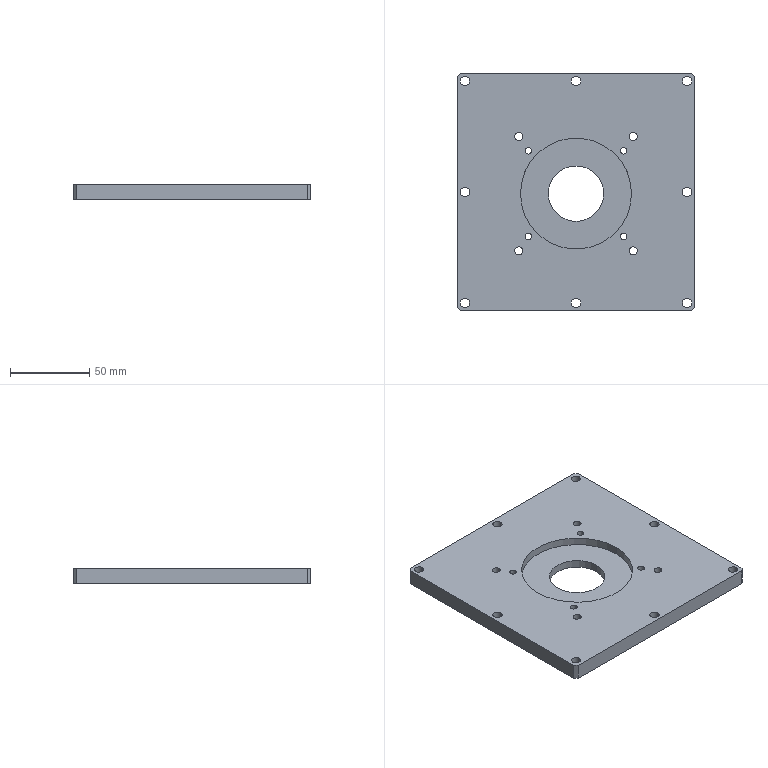Part | SolidWorks | features HoleWzd 3, ICE 2, Chamfer 1, Extrusion 1 | 1 solid | 47 faces | box 150 x 150 x 10 mm | volume 197414 mm3 | cylinder 36 | plane 11 | commonest cylinder face diameters 5.8 x16 4.2 x8 5 x8 35 x2 70 x2
STEP:
#1=CARTESIAN_POINT('',(32.1,26.,5.));
#2=VERTEX_POINT('',#1);
#3=CARTESIAN_POINT('',(27.9,26.,5.));
#4=VERTEX_POINT('',#3);
#5=CARTESIAN_POINT('',(30.,26.,5.));
#6=DIRECTION('',(0.,0.,-1.));
#7=DIRECTION('',(-1.,0.,0.));
#8=AXIS2_PLACEMENT_3D('',#5,#6,#7);
#9=CIRCLE('',#8,2.1);
#10=EDGE_CURVE('',#2,#4,#9,.T.);
#11=ORIENTED_EDGE('',*,*,#10,.F.);
#12=CARTESIAN_POINT('',(32.1,26.,-5.));
#13=VERTEX_POINT('',#12);
#14=CARTESIAN_POINT('',(32.1,26.,-5.));
#15=DIRECTION('',(0.,0.,-1.));
#16=VECTOR('',#15,1000.);
#17=LINE('',#14,#16);
#18=EDGE_CURVE('',#2,#13,#17,.T.);
#19=ORIENTED_EDGE('',*,*,#18,.T.);
#20=CARTESIAN_POINT('',(27.9,26.,-5.));
#21=VERTEX_POINT('',#20);
#22=CARTESIAN_POINT('',(30.,26.,-5.));
#23=DIRECTION('',(0.,0.,-1.));
#24=DIRECTION('',(-1.,0.,0.));
#25=AXIS2_PLACEMENT_3D('',#22,#23,#24);
#26=CIRCLE('',#25,2.1);
#27=EDGE_CURVE('',#13,#21,#26,.T.);
#28=ORIENTED_EDGE('',*,*,#27,.T.);
#29=CARTESIAN_POINT('',(27.9,26.,-5.));
#30=DIRECTION('',(0.,0.,-1.));
#31=VECTOR('',#30,1000.);
#32=LINE('',#29,#31);
#33=EDGE_CURVE('',#4,#21,#32,.T.);
#34=ORIENTED_EDGE('',*,*,#33,.F.);
#35=EDGE_LOOP('',(#11,#19,#28,#34));
#36=FACE_OUTER_BOUND('',#35,.T.);
#37=CARTESIAN_POINT('',(30.,26.,-5.));
#38=DIRECTION('',(0.,0.,-1.));
#39=DIRECTION('',(-1.,0.,0.));
#40=AXIS2_PLACEMENT_3D('',#37,#38,#39);
#41=CYLINDRICAL_SURFACE('',#40,2.1);
#42=ADVANCED_FACE('',(#36),#41,.F.);
#43=CARTESIAN_POINT('',(-27.9,26.,5.));
#44=VERTEX_POINT('',#43);
#45=CARTESIAN_POINT('',(-32.1,26.,5.));
#46=VERTEX_POINT('',#45);
#47=CARTESIAN_POINT('',(-30.,26.,5.));
#48=DIRECTION('',(0.,0.,-1.));
#49=DIRECTION('',(-1.,0.,0.));
#50=AXIS2_PLACEMENT_3D('',#47,#48,#49);
#51=CIRCLE('',#50,2.1);
#52=EDGE_CURVE('',#44,#46,#51,.T.);
#53=ORIENTED_EDGE('',*,*,#52,.F.);
#54=CARTESIAN_POINT('',(-27.9,26.,-5.));
#55=VERTEX_POINT('',#54);
#56=CARTESIAN_POINT('',(-27.9,26.,-5.));
#57=DIRECTION('',(0.,0.,-1.));
#58=VECTOR('',#57,1000.);
#59=LINE('',#56,#58);
#60=EDGE_CURVE('',#44,#55,#59,.T.);
#61=ORIENTED_EDGE('',*,*,#60,.T.);
#62=CARTESIAN_POINT('',(-32.1,26.,-5.));
#63=VERTEX_POINT('',#62);
#64=CARTESIAN_POINT('',(-30.,26.,-5.));
#65=DIRECTION('',(0.,0.,-1.));
#66=DIRECTION('',(-1.,0.,0.));
#67=AXIS2_PLACEMENT_3D('',#64,#65,#66);
#68=CIRCLE('',#67,2.1);
#69=EDGE_CURVE('',#55,#63,#68,.T.);
#70=ORIENTED_EDGE('',*,*,#69,.T.);
#71=CARTESIAN_POINT('',(-32.1,26.,-5.));
#72=DIRECTION('',(0.,0.,-1.));
#73=VECTOR('',#72,1000.);
#74=LINE('',#71,#73);
#75=EDGE_CURVE('',#46,#63,#74,.T.);
#76=ORIENTED_EDGE('',*,*,#75,.F.);
#77=EDGE_LOOP('',(#53,#61,#70,#76));
#78=FACE_OUTER_BOUND('',#77,.T.);
#79=CARTESIAN_POINT('',(-30.,26.,-5.));
#80=DIRECTION('',(0.,0.,-1.));
#81=DIRECTION('',(-1.,0.,0.));
#82=AXIS2_PLACEMENT_3D('',#79,#80,#81);
#83=CYLINDRICAL_SURFACE('',#82,2.1);
#84=ADVANCED_FACE('',(#78),#83,.F.);
#85=CARTESIAN_POINT('',(32.1,-28.,5.));
#86=VERTEX_POINT('',#85);
#87=CARTESIAN_POINT('',(27.9,-28.,5.));
#88=VERTEX_POINT('',#87);
#89=CARTESIAN_POINT('',(30.,-28.,5.));
#90=DIRECTION('',(0.,0.,-1.));
#91=DIRECTION('',(-1.,0.,0.));
#92=AXIS2_PLACEMENT_3D('',#89,#90,#91);
#93=CIRCLE('',#92,2.1);
#94=EDGE_CURVE('',#86,#88,#93,.T.);
#95=ORIENTED_EDGE('',*,*,#94,.F.);
#96=CARTESIAN_POINT('',(32.1,-28.,-5.));
#97=VERTEX_POINT('',#96);
#98=CARTESIAN_POINT('',(32.1,-28.,-5.));
#99=DIRECTION('',(0.,0.,-1.));
#100=VECTOR('',#99,1000.);
#101=LINE('',#98,#100);
#102=EDGE_CURVE('',#86,#97,#101,.T.);
#103=ORIENTED_EDGE('',*,*,#102,.T.);
#104=CARTESIAN_POINT('',(27.9,-28.,-5.));
#105=VERTEX_POINT('',#104);
#106=CARTESIAN_POINT('',(30.,-28.,-5.));
#107=DIRECTION('',(0.,0.,-1.));
#108=DIRECTION('',(-1.,0.,0.));
#109=AXIS2_PLACEMENT_3D('',#106,#107,#108);
#110=CIRCLE('',#109,2.1);
#111=EDGE_CURVE('',#97,#105,#110,.T.);
#112=ORIENTED_EDGE('',*,*,#111,.T.);
#113=CARTESIAN_POINT('',(27.9,-28.,-5.));
#114=DIRECTION('',(0.,0.,-1.));
#115=VECTOR('',#114,1000.);
#116=LINE('',#113,#115);
#117=EDGE_CURVE('',#88,#105,#116,.T.);
#118=ORIENTED_EDGE('',*,*,#117,.F.);
#119=EDGE_LOOP('',(#95,#103,#112,#118));
#120=FACE_OUTER_BOUND('',#119,.T.);
#121=CARTESIAN_POINT('',(30.,-28.,-5.));
#122=DIRECTION('',(0.,0.,-1.));
#123=DIRECTION('',(-1.,0.,0.));
#124=AXIS2_PLACEMENT_3D('',#121,#122,#123);
#125=CYLINDRICAL_SURFACE('',#124,2.1);
#126=ADVANCED_FACE('',(#120),#125,.F.);
#127=CARTESIAN_POINT('',(-27.9,-28.,5.));
#128=VERTEX_POINT('',#127);
#129=CARTESIAN_POINT('',(-32.1,-28.,5.));
#130=VERTEX_POINT('',#129);
#131=CARTESIAN_POINT('',(-30.,-28.,5.));
#132=DIRECTION('',(0.,0.,-1.));
#133=DIRECTION('',(-1.,0.,0.));
#134=AXIS2_PLACEMENT_3D('',#131,#132,#133);
#135=CIRCLE('',#134,2.1);
#136=EDGE_CURVE('',#128,#130,#135,.T.);
#137=ORIENTED_EDGE('',*,*,#136,.F.);
#138=CARTESIAN_POINT('',(-27.9,-28.,-5.));
#139=VERTEX_POINT('',#138);
#140=CARTESIAN_POINT('',(-27.9,-28.,-5.));
#141=DIRECTION('',(0.,0.,-1.));
#142=VECTOR('',#141,1000.);
#143=LINE('',#140,#142);
#144=EDGE_CURVE('',#128,#139,#143,.T.);
#145=ORIENTED_EDGE('',*,*,#144,.T.);
#146=CARTESIAN_POINT('',(-32.1,-28.,-5.));
#147=VERTEX_POINT('',#146);
#148=CARTESIAN_POINT('',(-30.,-28.,-5.));
#149=DIRECTION('',(0.,0.,-1.));
#150=DIRECTION('',(-1.,0.,0.));
#151=AXIS2_PLACEMENT_3D('',#148,#149,#150);
#152=CIRCLE('',#151,2.1);
#153=EDGE_CURVE('',#139,#147,#152,.T.);
#154=ORIENTED_EDGE('',*,*,#153,.T.);
#155=CARTESIAN_POINT('',(-32.1,-28.,-5.));
#156=DIRECTION('',(0.,0.,-1.));
#157=VECTOR('',#156,1000.);
#158=LINE('',#155,#157);
#159=EDGE_CURVE('',#130,#147,#158,.T.);
#160=ORIENTED_EDGE('',*,*,#159,.F.);
#161=EDGE_LOOP('',(#137,#145,#154,#160));
#162=FACE_OUTER_BOUND('',#161,.T.);
#163=CARTESIAN_POINT('',(-30.,-28.,-5.));
#164=DIRECTION('',(0.,0.,-1.));
#165=DIRECTION('',(-1.,0.,0.));
#166=AXIS2_PLACEMENT_3D('',#163,#164,#165);
#167=CYLINDRICAL_SURFACE('',#166,2.1);
#168=ADVANCED_FACE('',(#162),#167,.F.);
#169=CARTESIAN_POINT('',(-33.56,35.06,-5.));
#170=VERTEX_POINT('',#169);
#171=CARTESIAN_POINT('',(-38.56,35.06,-5.));
#172=VERTEX_POINT('',#171);
#173=CARTESIAN_POINT('',(-36.06,35.06,-5.));
#174=DIRECTION('',(0.,0.,-1.));
#175=DIRECTION('',(-1.,0.,0.));
#176=AXIS2_PLACEMENT_3D('',#173,#174,#175);
#177=CIRCLE('',#176,2.5);
#178=EDGE_CURVE('',#170,#172,#177,.T.);
#179=ORIENTED_EDGE('',*,*,#178,.T.);
#180=CARTESIAN_POINT('',(-38.56,35.06,5.));
#181=VERTEX_POINT('',#180);
#182=CARTESIAN_POINT('',(-38.56,35.06,5.));
#183=DIRECTION('',(0.,0.,1.));
#184=VECTOR('',#183,1000.);
#185=LINE('',#182,#184);
#186=EDGE_CURVE('',#172,#181,#185,.T.);
#187=ORIENTED_EDGE('',*,*,#186,.T.);
#188=CARTESIAN_POINT('',(-33.56,35.06,5.));
#189=VERTEX_POINT('',#188);
#190=CARTESIAN_POINT('',(-36.06,35.06,5.));
#191=DIRECTION('',(0.,0.,1.));
#192=DIRECTION('',(1.,0.,0.));
#193=AXIS2_PLACEMENT_3D('',#190,#191,#192);
#194=CIRCLE('',#193,2.5);
#195=EDGE_CURVE('',#181,#189,#194,.T.);
#196=ORIENTED_EDGE('',*,*,#195,.T.);
#197=CARTESIAN_POINT('',(-33.56,35.06,5.));
#198=DIRECTION('',(0.,0.,1.));
#199=VECTOR('',#198,1000.);
#200=LINE('',#197,#199);
#201=EDGE_CURVE('',#170,#189,#200,.T.);
#202=ORIENTED_EDGE('',*,*,#201,.F.);
#203=EDGE_LOOP('',(#179,#187,#196,#202));
#204=FACE_OUTER_BOUND('',#203,.T.);
#205=CARTESIAN_POINT('',(-36.06,35.06,5.));
#206=DIRECTION('',(0.,0.,1.));
#207=DIRECTION('',(1.,0.,0.));
#208=AXIS2_PLACEMENT_3D('',#205,#206,#207);
#209=CYLINDRICAL_SURFACE('',#208,2.5);
#210=ADVANCED_FACE('',(#204),#209,.F.);
#211=CARTESIAN_POINT('',(38.56,-37.06,-5.));
#212=VERTEX_POINT('',#211);
#213=CARTESIAN_POINT('',(33.56,-37.06,-5.));
#214=VERTEX_POINT('',#213);
#215=CARTESIAN_POINT('',(36.06,-37.06,-5.));
#216=DIRECTION('',(0.,0.,-1.));
#217=DIRECTION('',(-1.,0.,0.));
#218=AXIS2_PLACEMENT_3D('',#215,#216,#217);
#219=CIRCLE('',#218,2.5);
#220=EDGE_CURVE('',#212,#214,#219,.T.);
#221=ORIENTED_EDGE('',*,*,#220,.T.);
#222=CARTESIAN_POINT('',(33.56,-37.06,5.));
#223=VERTEX_POINT('',#222);
#224=CARTESIAN_POINT('',(33.56,-37.06,5.));
#225=DIRECTION('',(0.,0.,1.));
#226=VECTOR('',#225,1000.);
#227=LINE('',#224,#226);
#228=EDGE_CURVE('',#214,#223,#227,.T.);
#229=ORIENTED_EDGE('',*,*,#228,.T.);
#230=CARTESIAN_POINT('',(38.56,-37.06,5.));
#231=VERTEX_POINT('',#230);
#232=CARTESIAN_POINT('',(36.06,-37.06,5.));
#233=DIRECTION('',(0.,0.,1.));
#234=DIRECTION('',(1.,0.,0.));
#235=AXIS2_PLACEMENT_3D('',#232,#233,#234);
#236=CIRCLE('',#235,2.5);
#237=EDGE_CURVE('',#223,#231,#236,.T.);
#238=ORIENTED_EDGE('',*,*,#237,.T.);
#239=CARTESIAN_POINT('',(38.56,-37.06,5.));
#240=DIRECTION('',(0.,0.,1.));
#241=VECTOR('',#240,1000.);
#242=LINE('',#239,#241);
#243=EDGE_CURVE('',#212,#231,#242,.T.);
#244=ORIENTED_EDGE('',*,*,#243,.F.);
#245=EDGE_LOOP('',(#221,#229,#238,#244));
#246=FACE_OUTER_BOUND('',#245,.T.);
#247=CARTESIAN_POINT('',(36.06,-37.06,5.));
#248=DIRECTION('',(0.,0.,1.));
#249=DIRECTION('',(1.,0.,0.));
#250=AXIS2_PLACEMENT_3D('',#247,#248,#249);
#251=CYLINDRICAL_SURFACE('',#250,2.5);
#252=ADVANCED_FACE('',(#246),#251,.F.);
#253=CARTESIAN_POINT('',(38.56,35.06,-5.));
#254=VERTEX_POINT('',#253);
#255=CARTESIAN_POINT('',(33.56,35.06,-5.));
#256=VERTEX_POINT('',#255);
#257=CARTESIAN_POINT('',(36.06,35.06,-5.));
#258=DIRECTION('',(0.,0.,-1.));
#259=DIRECTION('',(-1.,0.,0.));
#260=AXIS2_PLACEMENT_3D('',#257,#258,#259);
#261=CIRCLE('',#260,2.5);
#262=EDGE_CURVE('',#254,#256,#261,.T.);
#263=ORIENTED_EDGE('',*,*,#262,.T.);
#264=CARTESIAN_POINT('',(33.56,35.06,5.));
#265=VERTEX_POINT('',#264);
#266=CARTESIAN_POINT('',(33.56,35.06,5.));
#267=DIRECTION('',(0.,0.,1.));
#268=VECTOR('',#267,1000.);
#269=LINE('',#266,#268);
#270=EDGE_CURVE('',#256,#265,#269,.T.);
#271=ORIENTED_EDGE('',*,*,#270,.T.);
#272=CARTESIAN_POINT('',(38.56,35.06,5.));
#273=VERTEX_POINT('',#272);
#274=CARTESIAN_POINT('',(36.06,35.06,5.));
#275=DIRECTION('',(0.,0.,1.));
#276=DIRECTION('',(1.,0.,0.));
#277=AXIS2_PLACEMENT_3D('',#274,#275,#276);
#278=CIRCLE('',#277,2.5);
#279=EDGE_CURVE('',#265,#273,#278,.T.);
#280=ORIENTED_EDGE('',*,*,#279,.T.);
#281=CARTESIAN_POINT('',(38.56,35.06,5.));
#282=DIRECTION('',(0.,0.,1.));
#283=VECTOR('',#282,1000.);
#284=LINE('',#281,#283);
#285=EDGE_CURVE('',#254,#273,#284,.T.);
#286=ORIENTED_EDGE('',*,*,#285,.F.);
#287=EDGE_LOOP('',(#263,#271,#280,#286));
#288=FACE_OUTER_BOUND('',#287,.T.);
#289=CARTESIAN_POINT('',(36.06,35.06,5.));
#290=DIRECTION('',(0.,0.,1.));
#291=DIRECTION('',(1.,0.,0.));
#292=AXIS2_PLACEMENT_3D('',#289,#290,#291);
#293=CYLINDRICAL_SURFACE('',#292,2.5);
#294=ADVANCED_FACE('',(#288),#293,.F.);
#295=CARTESIAN_POINT('',(-33.56,-37.06,-5.));
#296=VERTEX_POINT('',#295);
#297=CARTESIAN_POINT('',(-38.56,-37.06,-5.));
#298=VERTEX_POINT('',#297);
#299=CARTESIAN_POINT('',(-36.06,-37.06,-5.));
#300=DIRECTION('',(0.,0.,-1.));
#301=DIRECTION('',(-1.,0.,0.));
#302=AXIS2_PLACEMENT_3D('',#299,#300,#301);
#303=CIRCLE('',#302,2.5);
#304=EDGE_CURVE('',#296,#298,#303,.T.);
#305=ORIENTED_EDGE('',*,*,#304,.T.);
#306=CARTESIAN_POINT('',(-38.56,-37.06,5.));
#307=VERTEX_POINT('',#306);
#308=CARTESIAN_POINT('',(-38.56,-37.06,5.));
#309=DIRECTION('',(0.,0.,1.));
#310=VECTOR('',#309,1000.);
#311=LINE('',#308,#310);
#312=EDGE_CURVE('',#298,#307,#311,.T.);
#313=ORIENTED_EDGE('',*,*,#312,.T.);
#314=CARTESIAN_POINT('',(-33.56,-37.06,5.));
#315=VERTEX_POINT('',#314);
#316=CARTESIAN_POINT('',(-36.06,-37.06,5.));
#317=DIRECTION('',(0.,0.,1.));
#318=DIRECTION('',(1.,0.,0.));
#319=AXIS2_PLACEMENT_3D('',#316,#317,#318);
#320=CIRCLE('',#319,2.5);
#321=EDGE_CURVE('',#307,#315,#320,.T.);
#322=ORIENTED_EDGE('',*,*,#321,.T.);
#323=CARTESIAN_POINT('',(-33.56,-37.06,5.));
#324=DIRECTION('',(0.,0.,1.));
#325=VECTOR('',#324,1000.);
#326=LINE('',#323,#325);
#327=EDGE_CURVE('',#296,#315,#326,.T.);
#328=ORIENTED_EDGE('',*,*,#327,.F.);
#329=EDGE_LOOP('',(#305,#313,#322,#328));
#330=FACE_OUTER_BOUND('',#329,.T.);
#331=CARTESIAN_POINT('',(-36.06,-37.06,5.));
#332=DIRECTION('',(0.,0.,1.));
#333=DIRECTION('',(1.,0.,0.));
#334=AXIS2_PLACEMENT_3D('',#331,#332,#333);
#335=CYLINDRICAL_SURFACE('',#334,2.5);
#336=ADVANCED_FACE('',(#330),#335,.F.);
#337=CARTESIAN_POINT('',(-35.,-1.,0.));
#338=VERTEX_POINT('',#337);
#339=CARTESIAN_POINT('',(35.,-1.,0.));
#340=VERTEX_POINT('',#339);
#341=CARTESIAN_POINT('',(0.,-1.,0.));
#342=DIRECTION('',(0.,0.,1.));
#343=DIRECTION('',(1.,0.,0.));
#344=AXIS2_PLACEMENT_3D('',#341,#342,#343);
#345=CIRCLE('',#344,35.);
#346=EDGE_CURVE('',#338,#340,#345,.T.);
#347=ORIENTED_EDGE('',*,*,#346,.F.);
#348=CARTESIAN_POINT('',(-35.,-1.,5.));
#349=VERTEX_POINT('',#348);
#350=CARTESIAN_POINT('',(-35.,-1.,0.));
#351=DIRECTION('',(0.,0.,1.));
#352=VECTOR('',#351,1000.);
#353=LINE('',#350,#352);
#354=EDGE_CURVE('',#338,#349,#353,.T.);
#355=ORIENTED_EDGE('',*,*,#354,.T.);
#356=CARTESIAN_POINT('',(35.,-1.,5.));
#357=VERTEX_POINT('',#356);
#358=CARTESIAN_POINT('',(0.,-1.,5.));
#359=DIRECTION('',(0.,0.,1.));
#360=DIRECTION('',(1.,0.,0.));
#361=AXIS2_PLACEMENT_3D('',#358,#359,#360);
#362=CIRCLE('',#361,35.);
#363=EDGE_CURVE('',#349,#357,#362,.T.);
#364=ORIENTED_EDGE('',*,*,#363,.T.);
#365=CARTESIAN_POINT('',(35.,-1.,0.));
#366=DIRECTION('',(0.,0.,1.));
#367=VECTOR('',#366,1000.);
#368=LINE('',#365,#367);
#369=EDGE_CURVE('',#340,#357,#368,.T.);
#370=ORIENTED_EDGE('',*,*,#369,.F.);
#371=EDGE_LOOP('',(#347,#355,#364,#370));
#372=FACE_OUTER_BOUND('',#371,.T.);
#373=CARTESIAN_POINT('',(0.,-1.,0.));
#374=DIRECTION('',(0.,0.,1.));
#375=DIRECTION('',(1.,0.,0.));
#376=AXIS2_PLACEMENT_3D('',#373,#374,#375);
#377=CYLINDRICAL_SURFACE('',#376,35.);
#378=ADVANCED_FACE('',(#372),#377,.F.);
#379=CARTESIAN_POINT('',(72.9,70.,5.));
#380=VERTEX_POINT('',#379);
#381=CARTESIAN_POINT('',(67.1,70.,5.));
#382=VERTEX_POINT('',#381);
#383=CARTESIAN_POINT('',(70.,70.,5.));
#384=DIRECTION('',(0.,0.,-1.));
#385=DIRECTION('',(-1.,0.,0.));
#386=AXIS2_PLACEMENT_3D('',#383,#384,#385);
#387=CIRCLE('',#386,2.9);
#388=EDGE_CURVE('',#380,#382,#387,.T.);
#389=ORIENTED_EDGE('',*,*,#388,.F.);
#390=CARTESIAN_POINT('',(72.9,70.,-5.));
#391=VERTEX_POINT('',#390);
#392=CARTESIAN_POINT('',(72.9,70.,-5.));
#393=DIRECTION('',(0.,0.,-1.));
#394=VECTOR('',#393,1000.);
#395=LINE('',#392,#394);
#396=EDGE_CURVE('',#380,#391,#395,.T.);
#397=ORIENTED_EDGE('',*,*,#396,.T.);
#398=CARTESIAN_POINT('',(67.1,70.,-5.));
#399=VERTEX_POINT('',#398);
#400=CARTESIAN_POINT('',(70.,70.,-5.));
#401=DIRECTION('',(0.,0.,-1.));
#402=DIRECTION('',(-1.,0.,0.));
#403=AXIS2_PLACEMENT_3D('',#400,#401,#402);
#404=CIRCLE('',#403,2.9);
#405=EDGE_CURVE('',#391,#399,#404,.T.);
#406=ORIENTED_EDGE('',*,*,#405,.T.);
#407=CARTESIAN_POINT('',(67.1,70.,-5.));
#408=DIRECTION('',(0.,0.,-1.));
#409=VECTOR('',#408,1000.);
#410=LINE('',#407,#409);
#411=EDGE_CURVE('',#382,#399,#410,.T.);
#412=ORIENTED_EDGE('',*,*,#411,.F.);
#413=EDGE_LOOP('',(#389,#397,#406,#412));
#414=FACE_OUTER_BOUND('',#413,.T.);
#415=CARTESIAN_POINT('',(70.,70.,-5.));
#416=DIRECTION('',(0.,0.,-1.));
#417=DIRECTION('',(-1.,0.,0.));
#418=AXIS2_PLACEMENT_3D('',#415,#416,#417);
#419=CYLINDRICAL_SURFACE('',#418,2.9);
#420=ADVANCED_FACE('',(#414),#419,.F.);
#421=CARTESIAN_POINT('',(72.9,0.,5.));
#422=VERTEX_POINT('',#421);
#423=CARTESIAN_POINT('',(67.1,0.,5.));
#424=VERTEX_POINT('',#423);
#425=CARTESIAN_POINT('',(70.,0.,5.));
#426=DIRECTION('',(0.,0.,-1.));
#427=DIRECTION('',(-1.,0.,0.));
#428=AXIS2_PLACEMENT_3D('',#425,#426,#427);
#429=CIRCLE('',#428,2.9);
#430=EDGE_CURVE('',#422,#424,#429,.T.);
#431=ORIENTED_EDGE('',*,*,#430,.F.);
#432=CARTESIAN_POINT('',(72.9,0.,-5.));
#433=VERTEX_POINT('',#432);
#434=CARTESIAN_POINT('',(72.9,0.,-5.));
#435=DIRECTION('',(0.,0.,-1.));
#436=VECTOR('',#435,1000.);
#437=LINE('',#434,#436);
#438=EDGE_CURVE('',#422,#433,#437,.T.);
#439=ORIENTED_EDGE('',*,*,#438,.T.);
#440=CARTESIAN_POINT('',(67.1,0.,-5.));
#441=VERTEX_POINT('',#440);
#442=CARTESIAN_POINT('',(70.,0.,-5.));
#443=DIRECTION('',(0.,0.,-1.));
#444=DIRECTION('',(-1.,0.,0.));
#445=AXIS2_PLACEMENT_3D('',#442,#443,#444);
#446=CIRCLE('',#445,2.9);
#447=EDGE_CURVE('',#433,#441,#446,.T.);
#448=ORIENTED_EDGE('',*,*,#447,.T.);
#449=CARTESIAN_POINT('',(67.1,0.,-5.));
#450=DIRECTION('',(0.,0.,-1.));
#451=VECTOR('',#450,1000.);
#452=LINE('',#449,#451);
#453=EDGE_CURVE('',#424,#441,#452,.T.);
#454=ORIENTED_EDGE('',*,*,#453,.F.);
#455=EDGE_LOOP('',(#431,#439,#448,#454));
#456=FACE_OUTER_BOUND('',#455,.T.);
#457=CARTESIAN_POINT('',(70.,0.,-5.));
#458=DIRECTION('',(0.,0.,-1.));
#459=DIRECTION('',(-1.,0.,0.));
#460=AXIS2_PLACEMENT_3D('',#457,#458,#459);
#461=CYLINDRICAL_SURFACE('',#460,2.9);
#462=ADVANCED_FACE('',(#456),#461,.F.);
#463=CARTESIAN_POINT('',(72.9,-70.,5.));
#464=VERTEX_POINT('',#463);
#465=CARTESIAN_POINT('',(67.1,-70.,5.));
#466=VERTEX_POINT('',#465);
#467=CARTESIAN_POINT('',(70.,-70.,5.));
#468=DIRECTION('',(0.,0.,-1.));
#469=DIRECTION('',(-1.,0.,0.));
#470=AXIS2_PLACEMENT_3D('',#467,#468,#469);
#471=CIRCLE('',#470,2.9);
#472=EDGE_CURVE('',#464,#466,#471,.T.);
#473=ORIENTED_EDGE('',*,*,#472,.F.);
#474=CARTESIAN_POINT('',(72.9,-70.,-5.));
#475=VERTEX_POINT('',#474);
#476=CARTESIAN_POINT('',(72.9,-70.,-5.));
#477=DIRECTION('',(0.,0.,-1.));
#478=VECTOR('',#477,1000.);
#479=LINE('',#476,#478);
#480=EDGE_CURVE('',#464,#475,#479,.T.);
#481=ORIENTED_EDGE('',*,*,#480,.T.);
#482=CARTESIAN_POINT('',(67.1,-70.,-5.));
#483=VERTEX_POINT('',#482);
#484=CARTESIAN_POINT('',(70.,-70.,-5.));
#485=DIRECTION('',(0.,0.,-1.));
#486=DIRECTION('',(-1.,0.,0.));
#487=AXIS2_PLACEMENT_3D('',#484,#485,#486);
#488=CIRCLE('',#487,2.9);
#489=EDGE_CURVE('',#475,#483,#488,.T.);
#490=ORIENTED_EDGE('',*,*,#489,.T.);
#491=CARTESIAN_POINT('',(67.1,-70.,-5.));
#492=DIRECTION('',(0.,0.,-1.));
#493=VECTOR('',#492,1000.);
#494=LINE('',#491,#493);
#495=EDGE_CURVE('',#466,#483,#494,.T.);
#496=ORIENTED_EDGE('',*,*,#495,.F.);
#497=EDGE_LOOP('',(#473,#481,#490,#496));
#498=FACE_OUTER_BOUND('',#497,.T.);
#499=CARTESIAN_POINT('',(70.,-70.,-5.));
#500=DIRECTION('',(0.,0.,-1.));
#501=DIRECTION('',(-1.,0.,0.));
#502=AXIS2_PLACEMENT_3D('',#499,#500,#501);
#503=CYLINDRICAL_SURFACE('',#502,2.9);
#504=ADVANCED_FACE('',(#498),#503,.F.);
#505=CARTESIAN_POINT('',(2.9,-70.,5.));
#506=VERTEX_POINT('',#505);
#507=CARTESIAN_POINT('',(-2.9,-70.,5.));
#508=VERTEX_POINT('',#507);
#509=CARTESIAN_POINT('',(0.,-70.,5.));
#510=DIRECTION('',(0.,0.,-1.));
#511=DIRECTION('',(-1.,0.,0.));
#512=AXIS2_PLACEMENT_3D('',#509,#510,#511);
#513=CIRCLE('',#512,2.9);
#514=EDGE_CURVE('',#506,#508,#513,.T.);
#515=ORIENTED_EDGE('',*,*,#514,.F.);
#516=CARTESIAN_POINT('',(2.9,-70.,-5.));
#517=VERTEX_POINT('',#516);
#518=CARTESIAN_POINT('',(2.9,-70.,-5.));
#519=DIRECTION('',(0.,0.,-1.));
#520=VECTOR('',#519,1000.);
#521=LINE('',#518,#520);
#522=EDGE_CURVE('',#506,#517,#521,.T.);
#523=ORIENTED_EDGE('',*,*,#522,.T.);
#524=CARTESIAN_POINT('',(-2.9,-70.,-5.));
#525=VERTEX_POINT('',#524);
#526=CARTESIAN_POINT('',(0.,-70.,-5.));
#527=DIRECTION('',(0.,0.,-1.));
#528=DIRECTION('',(-1.,0.,0.));
#529=AXIS2_PLACEMENT_3D('',#526,#527,#528);
#530=CIRCLE('',#529,2.9);
#531=EDGE_CURVE('',#517,#525,#530,.T.);
#532=ORIENTED_EDGE('',*,*,#531,.T.);
#533=CARTESIAN_POINT('',(-2.9,-70.,-5.));
#534=DIRECTION('',(0.,0.,-1.));
#535=VECTOR('',#534,1000.);
#536=LINE('',#533,#535);
#537=EDGE_CURVE('',#508,#525,#536,.T.);
#538=ORIENTED_EDGE('',*,*,#537,.F.);
#539=EDGE_LOOP('',(#515,#523,#532,#538));
#540=FACE_OUTER_BOUND('',#539,.T.);
#541=CARTESIAN_POINT('',(0.,-70.,-5.));
#542=DIRECTION('',(0.,0.,-1.));
#543=DIRECTION('',(-1.,0.,0.));
#544=AXIS2_PLACEMENT_3D('',#541,#542,#543);
#545=CYLINDRICAL_SURFACE('',#544,2.9);
#546=ADVANCED_FACE('',(#540),#545,.F.);
#547=CARTESIAN_POINT('',(-67.1,-70.,5.));
#548=VERTEX_POINT('',#547);
#549=CARTESIAN_POINT('',(-72.9,-70.,5.));
#550=VERTEX_POINT('',#549);
#551=CARTESIAN_POINT('',(-70.,-70.,5.));
#552=DIRECTION('',(0.,0.,-1.));
#553=DIRECTION('',(-1.,0.,0.));
#554=AXIS2_PLACEMENT_3D('',#551,#552,#553);
#555=CIRCLE('',#554,2.9);
#556=EDGE_CURVE('',#548,#550,#555,.T.);
#557=ORIENTED_EDGE('',*,*,#556,.F.);
#558=CARTESIAN_POINT('',(-67.1,-70.,-5.));
#559=VERTEX_POINT('',#558);
#560=CARTESIAN_POINT('',(-67.1,-70.,-5.));
#561=DIRECTION('',(0.,0.,-1.));
#562=VECTOR('',#561,1000.);
#563=LINE('',#560,#562);
#564=EDGE_CURVE('',#548,#559,#563,.T.);
#565=ORIENTED_EDGE('',*,*,#564,.T.);
#566=CARTESIAN_POINT('',(-72.9,-70.,-5.));
#567=VERTEX_POINT('',#566);
#568=CARTESIAN_POINT('',(-70.,-70.,-5.));
#569=DIRECTION('',(0.,0.,-1.));
#570=DIRECTION('',(-1.,0.,0.));
#571=AXIS2_PLACEMENT_3D('',#568,#569,#570);
#572=CIRCLE('',#571,2.9);
#573=EDGE_CURVE('',#559,#567,#572,.T.);
#574=ORIENTED_EDGE('',*,*,#573,.T.);
#575=CARTESIAN_POINT('',(-72.9,-70.,-5.));
#576=DIRECTION('',(0.,0.,-1.));
#577=VECTOR('',#576,1000.);
#578=LINE('',#575,#577);
#579=EDGE_CURVE('',#550,#567,#578,.T.);
#580=ORIENTED_EDGE('',*,*,#579,.F.);
#581=EDGE_LOOP('',(#557,#565,#574,#580));
#582=FACE_OUTER_BOUND('',#581,.T.);
#583=CARTESIAN_POINT('',(-70.,-70.,-5.));
#584=DIRECTION('',(0.,0.,-1.));
#585=DIRECTION('',(-1.,0.,0.));
#586=AXIS2_PLACEMENT_3D('',#583,#584,#585);
#587=CYLINDRICAL_SURFACE('',#586,2.9);
#588=ADVANCED_FACE('',(#582),#587,.F.);
#589=CARTESIAN_POINT('',(-67.1,0.,5.));
#590=VERTEX_POINT('',#589);
#591=CARTESIAN_POINT('',(-72.9,0.,5.));
#592=VERTEX_POINT('',#591);
#593=CARTESIAN_POINT('',(-70.,0.,5.));
#594=DIRECTION('',(0.,0.,-1.));
#595=DIRECTION('',(-1.,0.,0.));
#596=AXIS2_PLACEMENT_3D('',#593,#594,#595);
#597=CIRCLE('',#596,2.9);
#598=EDGE_CURVE('',#590,#592,#597,.T.);
#599=ORIENTED_EDGE('',*,*,#598,.F.);
#600=CARTESIAN_POINT('',(-67.1,0.,-5.));
#601=VERTEX_POINT('',#600);
#602=CARTESIAN_POINT('',(-67.1,0.,-5.));
#603=DIRECTION('',(0.,0.,-1.));
#604=VECTOR('',#603,1000.);
#605=LINE('',#602,#604);
#606=EDGE_CURVE('',#590,#601,#605,.T.);
#607=ORIENTED_EDGE('',*,*,#606,.T.);
#608=CARTESIAN_POINT('',(-72.9,0.,-5.));
#609=VERTEX_POINT('',#608);
#610=CARTESIAN_POINT('',(-70.,0.,-5.));
#611=DIRECTION('',(0.,0.,-1.));
#612=DIRECTION('',(-1.,0.,0.));
#613=AXIS2_PLACEMENT_3D('',#610,#611,#612);
#614=CIRCLE('',#613,2.9);
#615=EDGE_CURVE('',#601,#609,#614,.T.);
#616=ORIENTED_EDGE('',*,*,#615,.T.);
#617=CARTESIAN_POINT('',(-72.9,0.,-5.));
#618=DIRECTION('',(0.,0.,-1.));
#619=VECTOR('',#618,1000.);
#620=LINE('',#617,#619);
#621=EDGE_CURVE('',#592,#609,#620,.T.);
#622=ORIENTED_EDGE('',*,*,#621,.F.);
#623=EDGE_LOOP('',(#599,#607,#616,#622));
#624=FACE_OUTER_BOUND('',#623,.T.);
#625=CARTESIAN_POINT('',(-70.,0.,-5.));
#626=DIRECTION('',(0.,0.,-1.));
#627=DIRECTION('',(-1.,0.,0.));
#628=AXIS2_PLACEMENT_3D('',#625,#626,#627);
#629=CYLINDRICAL_SURFACE('',#628,2.9);
#630=ADVANCED_FACE('',(#624),#629,.F.);
#631=CARTESIAN_POINT('',(-67.1,70.,5.));
#632=VERTEX_POINT('',#631);
#633=CARTESIAN_POINT('',(-72.9,70.,5.));
#634=VERTEX_POINT('',#633);
#635=CARTESIAN_POINT('',(-70.,70.,5.));
#636=DIRECTION('',(0.,0.,-1.));
#637=DIRECTION('',(-1.,0.,0.));
#638=AXIS2_PLACEMENT_3D('',#635,#636,#637);
#639=CIRCLE('',#638,2.9);
#640=EDGE_CURVE('',#632,#634,#639,.T.);
#641=ORIENTED_EDGE('',*,*,#640,.F.);
#642=CARTESIAN_POINT('',(-67.1,70.,-5.));
#643=VERTEX_POINT('',#642);
#644=CARTESIAN_POINT('',(-67.1,70.,-5.));
#645=DIRECTION('',(0.,0.,-1.));
#646=VECTOR('',#645,1000.);
#647=LINE('',#644,#646);
#648=EDGE_CURVE('',#632,#643,#647,.T.);
#649=ORIENTED_EDGE('',*,*,#648,.T.);
#650=CARTESIAN_POINT('',(-72.9,70.,-5.));
#651=VERTEX_POINT('',#650);
#652=CARTESIAN_POINT('',(-70.,70.,-5.));
#653=DIRECTION('',(0.,0.,-1.));
#654=DIRECTION('',(-1.,0.,0.));
#655=AXIS2_PLACEMENT_3D('',#652,#653,#654);
#656=CIRCLE('',#655,2.9);
#657=EDGE_CURVE('',#643,#651,#656,.T.);
#658=ORIENTED_EDGE('',*,*,#657,.T.);
#659=CARTESIAN_POINT('',(-72.9,70.,-5.));
#660=DIRECTION('',(0.,0.,-1.));
#661=VECTOR('',#660,1000.);
#662=LINE('',#659,#661);
#663=EDGE_CURVE('',#634,#651,#662,.T.);
#664=ORIENTED_EDGE('',*,*,#663,.F.);
#665=EDGE_LOOP('',(#641,#649,#658,#664));
#666=FACE_OUTER_BOUND('',#665,.T.);
#667=CARTESIAN_POINT('',(-70.,70.,-5.));
#668=DIRECTION('',(0.,0.,-1.));
#669=DIRECTION('',(-1.,0.,0.));
#670=AXIS2_PLACEMENT_3D('',#667,#668,#669);
#671=CYLINDRICAL_SURFACE('',#670,2.9);
#672=ADVANCED_FACE('',(#666),#671,.F.);
#673=CARTESIAN_POINT('',(2.9,70.,5.));
#674=VERTEX_POINT('',#673);
#675=CARTESIAN_POINT('',(-2.9,70.,5.));
#676=VERTEX_POINT('',#675);
#677=CARTESIAN_POINT('',(0.,70.,5.));
#678=DIRECTION('',(0.,0.,-1.));
#679=DIRECTION('',(-1.,0.,0.));
#680=AXIS2_PLACEMENT_3D('',#677,#678,#679);
#681=CIRCLE('',#680,2.9);
#682=EDGE_CURVE('',#674,#676,#681,.T.);
#683=ORIENTED_EDGE('',*,*,#682,.F.);
#684=CARTESIAN_POINT('',(2.9,70.,-5.));
#685=VERTEX_POINT('',#684);
#686=CARTESIAN_POINT('',(2.9,70.,-5.));
#687=DIRECTION('',(0.,0.,-1.));
#688=VECTOR('',#687,1000.);
#689=LINE('',#686,#688);
#690=EDGE_CURVE('',#674,#685,#689,.T.);
#691=ORIENTED_EDGE('',*,*,#690,.T.);
#692=CARTESIAN_POINT('',(-2.9,70.,-5.));
#693=VERTEX_POINT('',#692);
#694=CARTESIAN_POINT('',(0.,70.,-5.));
#695=DIRECTION('',(0.,0.,-1.));
#696=DIRECTION('',(-1.,0.,0.));
#697=AXIS2_PLACEMENT_3D('',#694,#695,#696);
#698=CIRCLE('',#697,2.9);
#699=EDGE_CURVE('',#685,#693,#698,.T.);
#700=ORIENTED_EDGE('',*,*,#699,.T.);
#701=CARTESIAN_POINT('',(-2.9,70.,-5.));
#702=DIRECTION('',(0.,0.,-1.));
#703=VECTOR('',#702,1000.);
#704=LINE('',#701,#703);
#705=EDGE_CURVE('',#676,#693,#704,.T.);
#706=ORIENTED_EDGE('',*,*,#705,.F.);
#707=EDGE_LOOP('',(#683,#691,#700,#706));
#708=FACE_OUTER_BOUND('',#707,.T.);
#709=CARTESIAN_POINT('',(0.,70.,-5.));
#710=DIRECTION('',(0.,0.,-1.));
#711=DIRECTION('',(-1.,0.,0.));
#712=AXIS2_PLACEMENT_3D('',#709,#710,#711);
#713=CYLINDRICAL_SURFACE('',#712,2.9);
#714=ADVANCED_FACE('',(#708),#713,.F.);
#715=CARTESIAN_POINT('',(17.5,-1.,0.));
#716=VERTEX_POINT('',#715);
#717=CARTESIAN_POINT('',(-17.5,-1.,0.));
#718=VERTEX_POINT('',#717);
#719=CARTESIAN_POINT('',(0.,-1.,0.));
#720=DIRECTION('',(0.,0.,-1.));
#721=DIRECTION('',(1.,0.,0.));
#722=AXIS2_PLACEMENT_3D('',#719,#720,#721);
#723=CIRCLE('',#722,17.5);
#724=EDGE_CURVE('',#716,#718,#723,.T.);
#725=ORIENTED_EDGE('',*,*,#724,.F.);
#726=CARTESIAN_POINT('',(17.5,-1.,-5.));
#727=VERTEX_POINT('',#726);
#728=CARTESIAN_POINT('',(17.5,-1.,5.));
#729=DIRECTION('',(0.,0.,-1.));
#730=VECTOR('',#729,1000.);
#731=LINE('',#728,#730);
#732=EDGE_CURVE('',#716,#727,#731,.T.);
#733=ORIENTED_EDGE('',*,*,#732,.T.);
#734=CARTESIAN_POINT('',(-17.5,-1.,-5.));
#735=VERTEX_POINT('',#734);
#736=CARTESIAN_POINT('',(0.,-1.,-5.));
#737=DIRECTION('',(0.,0.,-1.));
#738=DIRECTION('',(-1.,0.,0.));
#739=AXIS2_PLACEMENT_3D('',#736,#737,#738);
#740=CIRCLE('',#739,17.5);
#741=EDGE_CURVE('',#727,#735,#740,.T.);
#742=ORIENTED_EDGE('',*,*,#741,.T.);
#743=CARTESIAN_POINT('',(-17.5,-1.,5.));
#744=DIRECTION('',(0.,0.,-1.));
#745=VECTOR('',#744,1000.);
#746=LINE('',#743,#745);
#747=EDGE_CURVE('',#718,#735,#746,.T.);
#748=ORIENTED_EDGE('',*,*,#747,.F.);
#749=EDGE_LOOP('',(#725,#733,#742,#748));
#750=FACE_OUTER_BOUND('',#749,.T.);
#751=CARTESIAN_POINT('',(0.,-1.,5.));
#752=DIRECTION('',(0.,0.,-1.));
#753=DIRECTION('',(-1.,0.,0.));
#754=AXIS2_PLACEMENT_3D('',#751,#752,#753);
#755=CYLINDRICAL_SURFACE('',#754,17.5);
#756=ADVANCED_FACE('',(#750),#755,.F.);
#757=CARTESIAN_POINT('',(30.,26.,5.));
#758=DIRECTION('',(0.,0.,-1.));
#759=DIRECTION('',(-1.,0.,0.));
#760=AXIS2_PLACEMENT_3D('',#757,#758,#759);
#761=CIRCLE('',#760,2.1);
#762=EDGE_CURVE('',#4,#2,#761,.T.);
#763=ORIENTED_EDGE('',*,*,#762,.T.);
#764=ORIENTED_EDGE('',*,*,#10,.T.);
#765=EDGE_LOOP('',(#763,#764));
#766=FACE_BOUND('',#765,.T.);
#767=CARTESIAN_POINT('',(-30.,26.,5.));
#768=DIRECTION('',(0.,0.,-1.));
#769=DIRECTION('',(-1.,0.,0.));
#770=AXIS2_PLACEMENT_3D('',#767,#768,#769);
#771=CIRCLE('',#770,2.1);
#772=EDGE_CURVE('',#46,#44,#771,.T.);
#773=ORIENTED_EDGE('',*,*,#772,.T.);
#774=ORIENTED_EDGE('',*,*,#52,.T.);
#775=EDGE_LOOP('',(#773,#774));
#776=FACE_BOUND('',#775,.T.);
#777=CARTESIAN_POINT('',(30.,-28.,5.));
#778=DIRECTION('',(0.,0.,-1.));
#779=DIRECTION('',(-1.,0.,0.));
#780=AXIS2_PLACEMENT_3D('',#777,#778,#779);
#781=CIRCLE('',#780,2.1);
#782=EDGE_CURVE('',#88,#86,#781,.T.);
#783=ORIENTED_EDGE('',*,*,#782,.T.);
#784=ORIENTED_EDGE('',*,*,#94,.T.);
#785=EDGE_LOOP('',(#783,#784));
#786=FACE_BOUND('',#785,.T.);
#787=CARTESIAN_POINT('',(-30.,-28.,5.));
#788=DIRECTION('',(0.,0.,-1.));
#789=DIRECTION('',(-1.,0.,0.));
#790=AXIS2_PLACEMENT_3D('',#787,#788,#789);
#791=CIRCLE('',#790,2.1);
#792=EDGE_CURVE('',#130,#128,#791,.T.);
#793=ORIENTED_EDGE('',*,*,#792,.T.);
#794=ORIENTED_EDGE('',*,*,#136,.T.);
#795=EDGE_LOOP('',(#793,#794));
#796=FACE_BOUND('',#795,.T.);
#797=CARTESIAN_POINT('',(0.,-1.,5.));
#798=DIRECTION('',(0.,0.,1.));
#799=DIRECTION('',(1.,0.,0.));
#800=AXIS2_PLACEMENT_3D('',#797,#798,#799);
#801=CIRCLE('',#800,35.);
#802=EDGE_CURVE('',#357,#349,#801,.T.);
#803=ORIENTED_EDGE('',*,*,#802,.F.);
#804=ORIENTED_EDGE('',*,*,#363,.F.);
#805=EDGE_LOOP('',(#803,#804));
#806=FACE_BOUND('',#805,.T.);
#807=CARTESIAN_POINT('',(70.,70.,5.));
#808=DIRECTION('',(0.,0.,-1.));
#809=DIRECTION('',(-1.,0.,0.));
#810=AXIS2_PLACEMENT_3D('',#807,#808,#809);
#811=CIRCLE('',#810,2.9);
#812=EDGE_CURVE('',#382,#380,#811,.T.);
#813=ORIENTED_EDGE('',*,*,#812,.T.);
#814=ORIENTED_EDGE('',*,*,#388,.T.);
#815=EDGE_LOOP('',(#813,#814));
#816=FACE_BOUND('',#815,.T.);
#817=CARTESIAN_POINT('',(70.,0.,5.));
#818=DIRECTION('',(0.,0.,-1.));
#819=DIRECTION('',(-1.,0.,0.));
#820=AXIS2_PLACEMENT_3D('',#817,#818,#819);
#821=CIRCLE('',#820,2.9);
#822=EDGE_CURVE('',#424,#422,#821,.T.);
#823=ORIENTED_EDGE('',*,*,#822,.T.);
#824=ORIENTED_EDGE('',*,*,#430,.T.);
#825=EDGE_LOOP('',(#823,#824));
#826=FACE_BOUND('',#825,.T.);
#827=CARTESIAN_POINT('',(70.,-70.,5.));
#828=DIRECTION('',(0.,0.,-1.));
#829=DIRECTION('',(-1.,0.,0.));
#830=AXIS2_PLACEMENT_3D('',#827,#828,#829);
#831=CIRCLE('',#830,2.9);
#832=EDGE_CURVE('',#466,#464,#831,.T.);
#833=ORIENTED_EDGE('',*,*,#832,.T.);
#834=ORIENTED_EDGE('',*,*,#472,.T.);
#835=EDGE_LOOP('',(#833,#834));
#836=FACE_BOUND('',#835,.T.);
#837=CARTESIAN_POINT('',(0.,-70.,5.));
#838=DIRECTION('',(0.,0.,-1.));
#839=DIRECTION('',(-1.,0.,0.));
#840=AXIS2_PLACEMENT_3D('',#837,#838,#839);
#841=CIRCLE('',#840,2.9);
#842=EDGE_CURVE('',#508,#506,#841,.T.);
#843=ORIENTED_EDGE('',*,*,#842,.T.);
#844=ORIENTED_EDGE('',*,*,#514,.T.);
#845=EDGE_LOOP('',(#843,#844));
#846=FACE_BOUND('',#845,.T.);
#847=CARTESIAN_POINT('',(-70.,-70.,5.));
#848=DIRECTION('',(0.,0.,-1.));
#849=DIRECTION('',(-1.,0.,0.));
#850=AXIS2_PLACEMENT_3D('',#847,#848,#849);
#851=CIRCLE('',#850,2.9);
#852=EDGE_CURVE('',#550,#548,#851,.T.);
#853=ORIENTED_EDGE('',*,*,#852,.T.);
#854=ORIENTED_EDGE('',*,*,#556,.T.);
#855=EDGE_LOOP('',(#853,#854));
#856=FACE_BOUND('',#855,.T.);
#857=CARTESIAN_POINT('',(-70.,0.,5.));
#858=DIRECTION('',(0.,0.,-1.));
#859=DIRECTION('',(-1.,0.,0.));
#860=AXIS2_PLACEMENT_3D('',#857,#858,#859);
#861=CIRCLE('',#860,2.9);
#862=EDGE_CURVE('',#592,#590,#861,.T.);
#863=ORIENTED_EDGE('',*,*,#862,.T.);
#864=ORIENTED_EDGE('',*,*,#598,.T.);
#865=EDGE_LOOP('',(#863,#864));
#866=FACE_BOUND('',#865,.T.);
#867=CARTESIAN_POINT('',(-70.,70.,5.));
#868=DIRECTION('',(0.,0.,-1.));
#869=DIRECTION('',(-1.,0.,0.));
#870=AXIS2_PLACEMENT_3D('',#867,#868,#869);
#871=CIRCLE('',#870,2.9);
#872=EDGE_CURVE('',#634,#632,#871,.T.);
#873=ORIENTED_EDGE('',*,*,#872,.T.);
#874=ORIENTED_EDGE('',*,*,#640,.T.);
#875=EDGE_LOOP('',(#873,#874));
#876=FACE_BOUND('',#875,.T.);
#877=CARTESIAN_POINT('',(0.,70.,5.));
#878=DIRECTION('',(0.,0.,-1.));
#879=DIRECTION('',(-1.,0.,0.));
#880=AXIS2_PLACEMENT_3D('',#877,#878,#879);
#881=CIRCLE('',#880,2.9);
#882=EDGE_CURVE('',#676,#674,#881,.T.);
#883=ORIENTED_EDGE('',*,*,#882,.T.);
#884=ORIENTED_EDGE('',*,*,#682,.T.);
#885=EDGE_LOOP('',(#883,#884));
#886=FACE_BOUND('',#885,.T.);
#887=CARTESIAN_POINT('',(-75.,73.,5.));
#888=VERTEX_POINT('',#887);
#889=CARTESIAN_POINT('',(-75.,-73.,5.));
#890=VERTEX_POINT('',#889);
#891=CARTESIAN_POINT('',(-75.,-75.,5.));
#892=DIRECTION('',(0.,-1.,0.));
#893=VECTOR('',#892,1000.);
#894=LINE('',#891,#893);
#895=EDGE_CURVE('',#888,#890,#894,.T.);
#896=ORIENTED_EDGE('',*,*,#895,.T.);
#897=CARTESIAN_POINT('',(-73.,-75.,5.));
#898=VERTEX_POINT('',#897);
#899=CARTESIAN_POINT('',(-73.,-75.,5.));
#900=DIRECTION('',(0.7071,-0.7071,0.));
#901=VECTOR('',#900,1000.);
#902=LINE('',#899,#901);
#903=EDGE_CURVE('',#890,#898,#902,.T.);
#904=ORIENTED_EDGE('',*,*,#903,.T.);
#905=CARTESIAN_POINT('',(73.,-75.,5.));
#906=VERTEX_POINT('',#905);
#907=CARTESIAN_POINT('',(-75.,-75.,5.));
#908=DIRECTION('',(1.,0.,0.));
#909=VECTOR('',#908,1000.);
#910=LINE('',#907,#909);
#911=EDGE_CURVE('',#898,#906,#910,.T.);
#912=ORIENTED_EDGE('',*,*,#911,.T.);
#913=CARTESIAN_POINT('',(75.,-73.,5.));
#914=VERTEX_POINT('',#913);
#915=CARTESIAN_POINT('',(75.,-73.,5.));
#916=DIRECTION('',(0.7071,0.7071,0.));
#917=VECTOR('',#916,1000.);
#918=LINE('',#915,#917);
#919=EDGE_CURVE('',#906,#914,#918,.T.);
#920=ORIENTED_EDGE('',*,*,#919,.T.);
#921=CARTESIAN_POINT('',(75.,73.,5.));
#922=VERTEX_POINT('',#921);
#923=CARTESIAN_POINT('',(75.,-75.,5.));
#924=DIRECTION('',(0.,1.,0.));
#925=VECTOR('',#924,1000.);
#926=LINE('',#923,#925);
#927=EDGE_CURVE('',#914,#922,#926,.T.);
#928=ORIENTED_EDGE('',*,*,#927,.T.);
#929=CARTESIAN_POINT('',(73.,75.,5.));
#930=VERTEX_POINT('',#929);
#931=CARTESIAN_POINT('',(73.,75.,5.));
#932=DIRECTION('',(-0.7071,0.7071,0.));
#933=VECTOR('',#932,1000.);
#934=LINE('',#931,#933);
#935=EDGE_CURVE('',#922,#930,#934,.T.);
#936=ORIENTED_EDGE('',*,*,#935,.T.);
#937=CARTESIAN_POINT('',(-73.,75.,5.));
#938=VERTEX_POINT('',#937);
#939=CARTESIAN_POINT('',(-75.,75.,5.));
#940=DIRECTION('',(-1.,0.,0.));
#941=VECTOR('',#940,1000.);
#942=LINE('',#939,#941);
#943=EDGE_CURVE('',#930,#938,#942,.T.);
#944=ORIENTED_EDGE('',*,*,#943,.T.);
#945=CARTESIAN_POINT('',(-75.,73.,5.));
#946=DIRECTION('',(-0.7071,-0.7071,0.));
#947=VECTOR('',#946,1000.);
#948=LINE('',#945,#947);
#949=EDGE_CURVE('',#938,#888,#948,.T.);
#950=ORIENTED_EDGE('',*,*,#949,.T.);
#951=EDGE_LOOP('',(#896,#904,#912,#920,#928,#936,#944,#950));
#952=FACE_OUTER_BOUND('',#951,.T.);
#953=CARTESIAN_POINT('',(-36.06,-37.06,5.));
#954=DIRECTION('',(0.,0.,1.));
#955=DIRECTION('',(1.,0.,0.));
#956=AXIS2_PLACEMENT_3D('',#953,#954,#955);
#957=CIRCLE('',#956,2.5);
#958=EDGE_CURVE('',#315,#307,#957,.T.);
#959=ORIENTED_EDGE('',*,*,#958,.F.);
#960=ORIENTED_EDGE('',*,*,#321,.F.);
#961=EDGE_LOOP('',(#959,#960));
#962=FACE_BOUND('',#961,.T.);
#963=CARTESIAN_POINT('',(36.06,35.06,5.));
#964=DIRECTION('',(0.,0.,1.));
#965=DIRECTION('',(1.,0.,0.));
#966=AXIS2_PLACEMENT_3D('',#963,#964,#965);
#967=CIRCLE('',#966,2.5);
#968=EDGE_CURVE('',#273,#265,#967,.T.);
#969=ORIENTED_EDGE('',*,*,#968,.F.);
#970=ORIENTED_EDGE('',*,*,#279,.F.);
#971=EDGE_LOOP('',(#969,#970));
#972=FACE_BOUND('',#971,.T.);
#973=CARTESIAN_POINT('',(36.06,-37.06,5.));
#974=DIRECTION('',(0.,0.,1.));
#975=DIRECTION('',(1.,0.,0.));
#976=AXIS2_PLACEMENT_3D('',#973,#974,#975);
#977=CIRCLE('',#976,2.5);
#978=EDGE_CURVE('',#231,#223,#977,.T.);
#979=ORIENTED_EDGE('',*,*,#978,.F.);
#980=ORIENTED_EDGE('',*,*,#237,.F.);
#981=EDGE_LOOP('',(#979,#980));
#982=FACE_BOUND('',#981,.T.);
#983=CARTESIAN_POINT('',(-36.06,35.06,5.));
#984=DIRECTION('',(0.,0.,1.));
#985=DIRECTION('',(1.,0.,0.));
#986=AXIS2_PLACEMENT_3D('',#983,#984,#985);
#987=CIRCLE('',#986,2.5);
#988=EDGE_CURVE('',#189,#181,#987,.T.);
#989=ORIENTED_EDGE('',*,*,#988,.F.);
#990=ORIENTED_EDGE('',*,*,#195,.F.);
#991=EDGE_LOOP('',(#989,#990));
#992=FACE_BOUND('',#991,.T.);
#993=CARTESIAN_POINT('',(0.,0.,5.));
#994=DIRECTION('',(0.,0.,-1.));
#995=DIRECTION('',(-1.,0.,0.));
#996=AXIS2_PLACEMENT_3D('',#993,#994,#995);
#997=PLANE('',#996);
#998=ADVANCED_FACE('',(#766,#776,#786,#796,#806,#816,#826,#836,#846,#856,#866,#876,#886,#952,#962,#972,#982,#992),#997,.F.);
#999=ORIENTED_EDGE('',*,*,#732,.F.);
#1000=CARTESIAN_POINT('',(0.,-1.,0.));
#1001=DIRECTION('',(0.,0.,-1.));
#1002=DIRECTION('',(1.,0.,0.));
#1003=AXIS2_PLACEMENT_3D('',#1000,#1001,#1002);
#1004=CIRCLE('',#1003,17.5);
#1005=EDGE_CURVE('',#718,#716,#1004,.T.);
#1006=ORIENTED_EDGE('',*,*,#1005,.F.);
#1007=ORIENTED_EDGE('',*,*,#747,.T.);
#1008=CARTESIAN_POINT('',(0.,-1.,-5.));
#1009=DIRECTION('',(0.,0.,-1.));
#1010=DIRECTION('',(-1.,0.,0.));
#1011=AXIS2_PLACEMENT_3D('',#1008,#1009,#1010);
#1012=CIRCLE('',#1011,17.5);
#1013=EDGE_CURVE('',#735,#727,#1012,.T.);
#1014=ORIENTED_EDGE('',*,*,#1013,.T.);
#1015=EDGE_LOOP('',(#999,#1006,#1007,#1014));
#1016=FACE_OUTER_BOUND('',#1015,.T.);
#1017=CARTESIAN_POINT('',(0.,-1.,5.));
#1018=DIRECTION('',(0.,0.,-1.));
#1019=DIRECTION('',(-1.,0.,0.));
#1020=AXIS2_PLACEMENT_3D('',#1017,#1018,#1019);
#1021=CYLINDRICAL_SURFACE('',#1020,17.5);
#1022=ADVANCED_FACE('',(#1016),#1021,.F.);
#1023=ORIENTED_EDGE('',*,*,#927,.F.);
#1024=CARTESIAN_POINT('',(75.,-73.,-5.));
#1025=VERTEX_POINT('',#1024);
#1026=CARTESIAN_POINT('',(75.,-73.,5.));
#1027=DIRECTION('',(0.,0.,-1.));
#1028=VECTOR('',#1027,1000.);
#1029=LINE('',#1026,#1028);
#1030=EDGE_CURVE('',#914,#1025,#1029,.T.);
#1031=ORIENTED_EDGE('',*,*,#1030,.T.);
#1032=CARTESIAN_POINT('',(75.,73.,-5.));
#1033=VERTEX_POINT('',#1032);
#1034=CARTESIAN_POINT('',(75.,-75.,-5.));
#1035=DIRECTION('',(0.,1.,0.));
#1036=VECTOR('',#1035,1000.);
#1037=LINE('',#1034,#1036);
#1038=EDGE_CURVE('',#1025,#1033,#1037,.T.);
#1039=ORIENTED_EDGE('',*,*,#1038,.T.);
#1040=CARTESIAN_POINT('',(75.,73.,5.));
#1041=DIRECTION('',(0.,0.,1.));
#1042=VECTOR('',#1041,1000.);
#1043=LINE('',#1040,#1042);
#1044=EDGE_CURVE('',#1033,#922,#1043,.T.);
#1045=ORIENTED_EDGE('',*,*,#1044,.T.);
#1046=EDGE_LOOP('',(#1023,#1031,#1039,#1045));
#1047=FACE_OUTER_BOUND('',#1046,.T.);
#1048=CARTESIAN_POINT('',(75.,-75.,5.));
#1049=DIRECTION('',(-1.,0.,0.));
#1050=DIRECTION('',(0.,0.,1.));
#1051=AXIS2_PLACEMENT_3D('',#1048,#1049,#1050);
#1052=PLANE('',#1051);
#1053=ADVANCED_FACE('',(#1047),#1052,.F.);
#1054=ORIENTED_EDGE('',*,*,#943,.F.);
#1055=CARTESIAN_POINT('',(73.,75.,-5.));
#1056=VERTEX_POINT('',#1055);
#1057=CARTESIAN_POINT('',(73.,75.,5.));
#1058=DIRECTION('',(0.,0.,-1.));
#1059=VECTOR('',#1058,1000.);
#1060=LINE('',#1057,#1059);
#1061=EDGE_CURVE('',#930,#1056,#1060,.T.);
#1062=ORIENTED_EDGE('',*,*,#1061,.T.);
#1063=CARTESIAN_POINT('',(-73.,75.,-5.));
#1064=VERTEX_POINT('',#1063);
#1065=CARTESIAN_POINT('',(-75.,75.,-5.));
#1066=DIRECTION('',(-1.,0.,0.));
#1067=VECTOR('',#1066,1000.);
#1068=LINE('',#1065,#1067);
#1069=EDGE_CURVE('',#1056,#1064,#1068,.T.);
#1070=ORIENTED_EDGE('',*,*,#1069,.T.);
#1071=CARTESIAN_POINT('',(-73.,75.,5.));
#1072=DIRECTION('',(0.,0.,1.));
#1073=VECTOR('',#1072,1000.);
#1074=LINE('',#1071,#1073);
#1075=EDGE_CURVE('',#1064,#938,#1074,.T.);
#1076=ORIENTED_EDGE('',*,*,#1075,.T.);
#1077=EDGE_LOOP('',(#1054,#1062,#1070,#1076));
#1078=FACE_OUTER_BOUND('',#1077,.T.);
#1079=CARTESIAN_POINT('',(-75.,75.,5.));
#1080=DIRECTION('',(0.,-1.,0.));
#1081=DIRECTION('',(0.,0.,-1.));
#1082=AXIS2_PLACEMENT_3D('',#1079,#1080,#1081);
#1083=PLANE('',#1082);
#1084=ADVANCED_FACE('',(#1078),#1083,.F.);
#1085=CARTESIAN_POINT('',(-75.,73.,-5.));
#1086=VERTEX_POINT('',#1085);
#1087=CARTESIAN_POINT('',(-75.,-73.,-5.));
#1088=VERTEX_POINT('',#1087);
#1089=CARTESIAN_POINT('',(-75.,-75.,-5.));
#1090=DIRECTION('',(0.,-1.,0.));
#1091=VECTOR('',#1090,1000.);
#1092=LINE('',#1089,#1091);
#1093=EDGE_CURVE('',#1086,#1088,#1092,.T.);
#1094=ORIENTED_EDGE('',*,*,#1093,.T.);
#1095=CARTESIAN_POINT('',(-75.,-73.,5.));
#1096=DIRECTION('',(0.,0.,1.));
#1097=VECTOR('',#1096,1000.);
#1098=LINE('',#1095,#1097);
#1099=EDGE_CURVE('',#1088,#890,#1098,.T.);
#1100=ORIENTED_EDGE('',*,*,#1099,.T.);
#1101=ORIENTED_EDGE('',*,*,#895,.F.);
#1102=CARTESIAN_POINT('',(-75.,73.,5.));
#1103=DIRECTION('',(0.,0.,-1.));
#1104=VECTOR('',#1103,1000.);
#1105=LINE('',#1102,#1104);
#1106=EDGE_CURVE('',#888,#1086,#1105,.T.);
#1107=ORIENTED_EDGE('',*,*,#1106,.T.);
#1108=EDGE_LOOP('',(#1094,#1100,#1101,#1107));
#1109=FACE_OUTER_BOUND('',#1108,.T.);
#1110=CARTESIAN_POINT('',(-75.,-75.,5.));
#1111=DIRECTION('',(1.,0.,0.));
#1112=DIRECTION('',(0.,0.,-1.));
#1113=AXIS2_PLACEMENT_3D('',#1110,#1111,#1112);
#1114=PLANE('',#1113);
#1115=ADVANCED_FACE('',(#1109),#1114,.F.);
#1116=ORIENTED_EDGE('',*,*,#911,.F.);
#1117=CARTESIAN_POINT('',(-73.,-75.,-5.));
#1118=VERTEX_POINT('',#1117);
#1119=CARTESIAN_POINT('',(-73.,-75.,5.));
#1120=DIRECTION('',(0.,0.,-1.));
#1121=VECTOR('',#1120,1000.);
#1122=LINE('',#1119,#1121);
#1123=EDGE_CURVE('',#898,#1118,#1122,.T.);
#1124=ORIENTED_EDGE('',*,*,#1123,.T.);
#1125=CARTESIAN_POINT('',(73.,-75.,-5.));
#1126=VERTEX_POINT('',#1125);
#1127=CARTESIAN_POINT('',(-75.,-75.,-5.));
#1128=DIRECTION('',(1.,0.,0.));
#1129=VECTOR('',#1128,1000.);
#1130=LINE('',#1127,#1129);
#1131=EDGE_CURVE('',#1118,#1126,#1130,.T.);
#1132=ORIENTED_EDGE('',*,*,#1131,.T.);
#1133=CARTESIAN_POINT('',(73.,-75.,5.));
#1134=DIRECTION('',(0.,0.,1.));
#1135=VECTOR('',#1134,1000.);
#1136=LINE('',#1133,#1135);
#1137=EDGE_CURVE('',#1126,#906,#1136,.T.);
#1138=ORIENTED_EDGE('',*,*,#1137,.T.);
#1139=EDGE_LOOP('',(#1116,#1124,#1132,#1138));
#1140=FACE_OUTER_BOUND('',#1139,.T.);
#1141=CARTESIAN_POINT('',(-75.,-75.,5.));
#1142=DIRECTION('',(0.,1.,0.));
#1143=DIRECTION('',(0.,0.,1.));
#1144=AXIS2_PLACEMENT_3D('',#1141,#1142,#1143);
#1145=PLANE('',#1144);
#1146=ADVANCED_FACE('',(#1140),#1145,.F.);
#1147=CARTESIAN_POINT('',(30.,26.,-5.));
#1148=DIRECTION('',(0.,0.,-1.));
#1149=DIRECTION('',(-1.,0.,0.));
#1150=AXIS2_PLACEMENT_3D('',#1147,#1148,#1149);
#1151=CIRCLE('',#1150,2.1);
#1152=EDGE_CURVE('',#21,#13,#1151,.T.);
#1153=ORIENTED_EDGE('',*,*,#1152,.F.);
#1154=ORIENTED_EDGE('',*,*,#27,.F.);
#1155=EDGE_LOOP('',(#1153,#1154));
#1156=FACE_BOUND('',#1155,.T.);
#1157=CARTESIAN_POINT('',(-30.,26.,-5.));
#1158=DIRECTION('',(0.,0.,-1.));
#1159=DIRECTION('',(-1.,0.,0.));
#1160=AXIS2_PLACEMENT_3D('',#1157,#1158,#1159);
#1161=CIRCLE('',#1160,2.1);
#1162=EDGE_CURVE('',#63,#55,#1161,.T.);
#1163=ORIENTED_EDGE('',*,*,#1162,.F.);
#1164=ORIENTED_EDGE('',*,*,#69,.F.);
#1165=EDGE_LOOP('',(#1163,#1164));
#1166=FACE_BOUND('',#1165,.T.);
#1167=CARTESIAN_POINT('',(30.,-28.,-5.));
#1168=DIRECTION('',(0.,0.,-1.));
#1169=DIRECTION('',(-1.,0.,0.));
#1170=AXIS2_PLACEMENT_3D('',#1167,#1168,#1169);
#1171=CIRCLE('',#1170,2.1);
#1172=EDGE_CURVE('',#105,#97,#1171,.T.);
#1173=ORIENTED_EDGE('',*,*,#1172,.F.);
#1174=ORIENTED_EDGE('',*,*,#111,.F.);
#1175=EDGE_LOOP('',(#1173,#1174));
#1176=FACE_BOUND('',#1175,.T.);
#1177=CARTESIAN_POINT('',(-30.,-28.,-5.));
#1178=DIRECTION('',(0.,0.,-1.));
#1179=DIRECTION('',(-1.,0.,0.));
#1180=AXIS2_PLACEMENT_3D('',#1177,#1178,#1179);
#1181=CIRCLE('',#1180,2.1);
#1182=EDGE_CURVE('',#147,#139,#1181,.T.);
#1183=ORIENTED_EDGE('',*,*,#1182,.F.);
#1184=ORIENTED_EDGE('',*,*,#153,.F.);
#1185=EDGE_LOOP('',(#1183,#1184));
#1186=FACE_BOUND('',#1185,.T.);
#1187=ORIENTED_EDGE('',*,*,#178,.F.);
#1188=CARTESIAN_POINT('',(-36.06,35.06,-5.));
#1189=DIRECTION('',(0.,0.,-1.));
#1190=DIRECTION('',(-1.,0.,0.));
#1191=AXIS2_PLACEMENT_3D('',#1188,#1189,#1190);
#1192=CIRCLE('',#1191,2.5);
#1193=EDGE_CURVE('',#172,#170,#1192,.T.);
#1194=ORIENTED_EDGE('',*,*,#1193,.F.);
#1195=EDGE_LOOP('',(#1187,#1194));
#1196=FACE_BOUND('',#1195,.T.);
#1197=ORIENTED_EDGE('',*,*,#220,.F.);
#1198=CARTESIAN_POINT('',(36.06,-37.06,-5.));
#1199=DIRECTION('',(0.,0.,-1.));
#1200=DIRECTION('',(-1.,0.,0.));
#1201=AXIS2_PLACEMENT_3D('',#1198,#1199,#1200);
#1202=CIRCLE('',#1201,2.5);
#1203=EDGE_CURVE('',#214,#212,#1202,.T.);
#1204=ORIENTED_EDGE('',*,*,#1203,.F.);
#1205=EDGE_LOOP('',(#1197,#1204));
#1206=FACE_BOUND('',#1205,.T.);
#1207=ORIENTED_EDGE('',*,*,#262,.F.);
#1208=CARTESIAN_POINT('',(36.06,35.06,-5.));
#1209=DIRECTION('',(0.,0.,-1.));
#1210=DIRECTION('',(-1.,0.,0.));
#1211=AXIS2_PLACEMENT_3D('',#1208,#1209,#1210);
#1212=CIRCLE('',#1211,2.5);
#1213=EDGE_CURVE('',#256,#254,#1212,.T.);
#1214=ORIENTED_EDGE('',*,*,#1213,.F.);
#1215=EDGE_LOOP('',(#1207,#1214));
#1216=FACE_BOUND('',#1215,.T.);
#1217=ORIENTED_EDGE('',*,*,#304,.F.);
#1218=CARTESIAN_POINT('',(-36.06,-37.06,-5.));
#1219=DIRECTION('',(0.,0.,-1.));
#1220=DIRECTION('',(-1.,0.,0.));
#1221=AXIS2_PLACEMENT_3D('',#1218,#1219,#1220);
#1222=CIRCLE('',#1221,2.5);
#1223=EDGE_CURVE('',#298,#296,#1222,.T.);
#1224=ORIENTED_EDGE('',*,*,#1223,.F.);
#1225=EDGE_LOOP('',(#1217,#1224));
#1226=FACE_BOUND('',#1225,.T.);
#1227=CARTESIAN_POINT('',(70.,70.,-5.));
#1228=DIRECTION('',(0.,0.,-1.));
#1229=DIRECTION('',(-1.,0.,0.));
#1230=AXIS2_PLACEMENT_3D('',#1227,#1228,#1229);
#1231=CIRCLE('',#1230,2.9);
#1232=EDGE_CURVE('',#399,#391,#1231,.T.);
#1233=ORIENTED_EDGE('',*,*,#1232,.F.);
#1234=ORIENTED_EDGE('',*,*,#405,.F.);
#1235=EDGE_LOOP('',(#1233,#1234));
#1236=FACE_BOUND('',#1235,.T.);
#1237=CARTESIAN_POINT('',(70.,0.,-5.));
#1238=DIRECTION('',(0.,0.,-1.));
#1239=DIRECTION('',(-1.,0.,0.));
#1240=AXIS2_PLACEMENT_3D('',#1237,#1238,#1239);
#1241=CIRCLE('',#1240,2.9);
#1242=EDGE_CURVE('',#441,#433,#1241,.T.);
#1243=ORIENTED_EDGE('',*,*,#1242,.F.);
#1244=ORIENTED_EDGE('',*,*,#447,.F.);
#1245=EDGE_LOOP('',(#1243,#1244));
#1246=FACE_BOUND('',#1245,.T.);
#1247=CARTESIAN_POINT('',(70.,-70.,-5.));
#1248=DIRECTION('',(0.,0.,-1.));
#1249=DIRECTION('',(-1.,0.,0.));
#1250=AXIS2_PLACEMENT_3D('',#1247,#1248,#1249);
#1251=CIRCLE('',#1250,2.9);
#1252=EDGE_CURVE('',#483,#475,#1251,.T.);
#1253=ORIENTED_EDGE('',*,*,#1252,.F.);
#1254=ORIENTED_EDGE('',*,*,#489,.F.);
#1255=EDGE_LOOP('',(#1253,#1254));
#1256=FACE_BOUND('',#1255,.T.);
#1257=CARTESIAN_POINT('',(0.,-70.,-5.));
#1258=DIRECTION('',(0.,0.,-1.));
#1259=DIRECTION('',(-1.,0.,0.));
#1260=AXIS2_PLACEMENT_3D('',#1257,#1258,#1259);
#1261=CIRCLE('',#1260,2.9);
#1262=EDGE_CURVE('',#525,#517,#1261,.T.);
#1263=ORIENTED_EDGE('',*,*,#1262,.F.);
#1264=ORIENTED_EDGE('',*,*,#531,.F.);
#1265=EDGE_LOOP('',(#1263,#1264));
#1266=FACE_BOUND('',#1265,.T.);
#1267=CARTESIAN_POINT('',(-70.,-70.,-5.));
#1268=DIRECTION('',(0.,0.,-1.));
#1269=DIRECTION('',(-1.,0.,0.));
#1270=AXIS2_PLACEMENT_3D('',#1267,#1268,#1269);
#1271=CIRCLE('',#1270,2.9);
#1272=EDGE_CURVE('',#567,#559,#1271,.T.);
#1273=ORIENTED_EDGE('',*,*,#1272,.F.);
#1274=ORIENTED_EDGE('',*,*,#573,.F.);
#1275=EDGE_LOOP('',(#1273,#1274));
#1276=FACE_BOUND('',#1275,.T.);
#1277=CARTESIAN_POINT('',(-70.,0.,-5.));
#1278=DIRECTION('',(0.,0.,-1.));
#1279=DIRECTION('',(-1.,0.,0.));
#1280=AXIS2_PLACEMENT_3D('',#1277,#1278,#1279);
#1281=CIRCLE('',#1280,2.9);
#1282=EDGE_CURVE('',#609,#601,#1281,.T.);
#1283=ORIENTED_EDGE('',*,*,#1282,.F.);
#1284=ORIENTED_EDGE('',*,*,#615,.F.);
#1285=EDGE_LOOP('',(#1283,#1284));
#1286=FACE_BOUND('',#1285,.T.);
#1287=CARTESIAN_POINT('',(-70.,70.,-5.));
#1288=DIRECTION('',(0.,0.,-1.));
#1289=DIRECTION('',(-1.,0.,0.));
#1290=AXIS2_PLACEMENT_3D('',#1287,#1288,#1289);
#1291=CIRCLE('',#1290,2.9);
#1292=EDGE_CURVE('',#651,#643,#1291,.T.);
#1293=ORIENTED_EDGE('',*,*,#1292,.F.);
#1294=ORIENTED_EDGE('',*,*,#657,.F.);
#1295=EDGE_LOOP('',(#1293,#1294));
#1296=FACE_BOUND('',#1295,.T.);
#1297=CARTESIAN_POINT('',(0.,70.,-5.));
#1298=DIRECTION('',(0.,0.,-1.));
#1299=DIRECTION('',(-1.,0.,0.));
#1300=AXIS2_PLACEMENT_3D('',#1297,#1298,#1299);
#1301=CIRCLE('',#1300,2.9);
#1302=EDGE_CURVE('',#693,#685,#1301,.T.);
#1303=ORIENTED_EDGE('',*,*,#1302,.F.);
#1304=ORIENTED_EDGE('',*,*,#699,.F.);
#1305=EDGE_LOOP('',(#1303,#1304));
#1306=FACE_BOUND('',#1305,.T.);
#1307=ORIENTED_EDGE('',*,*,#1013,.F.);
#1308=ORIENTED_EDGE('',*,*,#741,.F.);
#1309=EDGE_LOOP('',(#1307,#1308));
#1310=FACE_BOUND('',#1309,.T.);
#1311=ORIENTED_EDGE('',*,*,#1131,.F.);
#1312=CARTESIAN_POINT('',(-74.,-74.,-5.));
#1313=DIRECTION('',(-0.7071,0.7071,0.));
#1314=VECTOR('',#1313,1000.);
#1315=LINE('',#1312,#1314);
#1316=EDGE_CURVE('',#1118,#1088,#1315,.T.);
#1317=ORIENTED_EDGE('',*,*,#1316,.T.);
#1318=ORIENTED_EDGE('',*,*,#1093,.F.);
#1319=CARTESIAN_POINT('',(-74.,74.,-5.));
#1320=DIRECTION('',(0.7071,0.7071,0.));
#1321=VECTOR('',#1320,1000.);
#1322=LINE('',#1319,#1321);
#1323=EDGE_CURVE('',#1086,#1064,#1322,.T.);
#1324=ORIENTED_EDGE('',*,*,#1323,.T.);
#1325=ORIENTED_EDGE('',*,*,#1069,.F.);
#1326=CARTESIAN_POINT('',(74.,74.,-5.));
#1327=DIRECTION('',(0.7071,-0.7071,0.));
#1328=VECTOR('',#1327,1000.);
#1329=LINE('',#1326,#1328);
#1330=EDGE_CURVE('',#1056,#1033,#1329,.T.);
#1331=ORIENTED_EDGE('',*,*,#1330,.T.);
#1332=ORIENTED_EDGE('',*,*,#1038,.F.);
#1333=CARTESIAN_POINT('',(74.,-74.,-5.));
#1334=DIRECTION('',(-0.7071,-0.7071,0.));
#1335=VECTOR('',#1334,1000.);
#1336=LINE('',#1333,#1335);
#1337=EDGE_CURVE('',#1025,#1126,#1336,.T.);
#1338=ORIENTED_EDGE('',*,*,#1337,.T.);
#1339=EDGE_LOOP('',(#1311,#1317,#1318,#1324,#1325,#1331,#1332,#1338));
#1340=FACE_OUTER_BOUND('',#1339,.T.);
#1341=CARTESIAN_POINT('',(0.,0.,-5.));
#1342=DIRECTION('',(0.,0.,-1.));
#1343=DIRECTION('',(-1.,0.,0.));
#1344=AXIS2_PLACEMENT_3D('',#1341,#1342,#1343);
#1345=PLANE('',#1344);
#1346=ADVANCED_FACE('',(#1156,#1166,#1176,#1186,#1196,#1206,#1216,#1226,#1236,#1246,#1256,#1266,#1276,#1286,#1296,#1306,#1310,#1340),#1345,.T.);
#1347=ORIENTED_EDGE('',*,*,#690,.F.);
#1348=ORIENTED_EDGE('',*,*,#882,.F.);
#1349=ORIENTED_EDGE('',*,*,#705,.T.);
#1350=ORIENTED_EDGE('',*,*,#1302,.T.);
#1351=EDGE_LOOP('',(#1347,#1348,#1349,#1350));
#1352=FACE_OUTER_BOUND('',#1351,.T.);
#1353=CARTESIAN_POINT('',(0.,70.,-5.));
#1354=DIRECTION('',(0.,0.,-1.));
#1355=DIRECTION('',(-1.,0.,0.));
#1356=AXIS2_PLACEMENT_3D('',#1353,#1354,#1355);
#1357=CYLINDRICAL_SURFACE('',#1356,2.9);
#1358=ADVANCED_FACE('',(#1352),#1357,.F.);
#1359=ORIENTED_EDGE('',*,*,#648,.F.);
#1360=ORIENTED_EDGE('',*,*,#872,.F.);
#1361=ORIENTED_EDGE('',*,*,#663,.T.);
#1362=ORIENTED_EDGE('',*,*,#1292,.T.);
#1363=EDGE_LOOP('',(#1359,#1360,#1361,#1362));
#1364=FACE_OUTER_BOUND('',#1363,.T.);
#1365=CARTESIAN_POINT('',(-70.,70.,-5.));
#1366=DIRECTION('',(0.,0.,-1.));
#1367=DIRECTION('',(-1.,0.,0.));
#1368=AXIS2_PLACEMENT_3D('',#1365,#1366,#1367);
#1369=CYLINDRICAL_SURFACE('',#1368,2.9);
#1370=ADVANCED_FACE('',(#1364),#1369,.F.);
#1371=ORIENTED_EDGE('',*,*,#606,.F.);
#1372=ORIENTED_EDGE('',*,*,#862,.F.);
#1373=ORIENTED_EDGE('',*,*,#621,.T.);
#1374=ORIENTED_EDGE('',*,*,#1282,.T.);
#1375=EDGE_LOOP('',(#1371,#1372,#1373,#1374));
#1376=FACE_OUTER_BOUND('',#1375,.T.);
#1377=CARTESIAN_POINT('',(-70.,0.,-5.));
#1378=DIRECTION('',(0.,0.,-1.));
#1379=DIRECTION('',(-1.,0.,0.));
#1380=AXIS2_PLACEMENT_3D('',#1377,#1378,#1379);
#1381=CYLINDRICAL_SURFACE('',#1380,2.9);
#1382=ADVANCED_FACE('',(#1376),#1381,.F.);
#1383=ORIENTED_EDGE('',*,*,#564,.F.);
#1384=ORIENTED_EDGE('',*,*,#852,.F.);
#1385=ORIENTED_EDGE('',*,*,#579,.T.);
#1386=ORIENTED_EDGE('',*,*,#1272,.T.);
#1387=EDGE_LOOP('',(#1383,#1384,#1385,#1386));
#1388=FACE_OUTER_BOUND('',#1387,.T.);
#1389=CARTESIAN_POINT('',(-70.,-70.,-5.));
#1390=DIRECTION('',(0.,0.,-1.));
#1391=DIRECTION('',(-1.,0.,0.));
#1392=AXIS2_PLACEMENT_3D('',#1389,#1390,#1391);
#1393=CYLINDRICAL_SURFACE('',#1392,2.9);
#1394=ADVANCED_FACE('',(#1388),#1393,.F.);
#1395=ORIENTED_EDGE('',*,*,#522,.F.);
#1396=ORIENTED_EDGE('',*,*,#842,.F.);
#1397=ORIENTED_EDGE('',*,*,#537,.T.);
#1398=ORIENTED_EDGE('',*,*,#1262,.T.);
#1399=EDGE_LOOP('',(#1395,#1396,#1397,#1398));
#1400=FACE_OUTER_BOUND('',#1399,.T.);
#1401=CARTESIAN_POINT('',(0.,-70.,-5.));
#1402=DIRECTION('',(0.,0.,-1.));
#1403=DIRECTION('',(-1.,0.,0.));
#1404=AXIS2_PLACEMENT_3D('',#1401,#1402,#1403);
#1405=CYLINDRICAL_SURFACE('',#1404,2.9);
#1406=ADVANCED_FACE('',(#1400),#1405,.F.);
#1407=ORIENTED_EDGE('',*,*,#480,.F.);
#1408=ORIENTED_EDGE('',*,*,#832,.F.);
#1409=ORIENTED_EDGE('',*,*,#495,.T.);
#1410=ORIENTED_EDGE('',*,*,#1252,.T.);
#1411=EDGE_LOOP('',(#1407,#1408,#1409,#1410));
#1412=FACE_OUTER_BOUND('',#1411,.T.);
#1413=CARTESIAN_POINT('',(70.,-70.,-5.));
#1414=DIRECTION('',(0.,0.,-1.));
#1415=DIRECTION('',(-1.,0.,0.));
#1416=AXIS2_PLACEMENT_3D('',#1413,#1414,#1415);
#1417=CYLINDRICAL_SURFACE('',#1416,2.9);
#1418=ADVANCED_FACE('',(#1412),#1417,.F.);
#1419=ORIENTED_EDGE('',*,*,#438,.F.);
#1420=ORIENTED_EDGE('',*,*,#822,.F.);
#1421=ORIENTED_EDGE('',*,*,#453,.T.);
#1422=ORIENTED_EDGE('',*,*,#1242,.T.);
#1423=EDGE_LOOP('',(#1419,#1420,#1421,#1422));
#1424=FACE_OUTER_BOUND('',#1423,.T.);
#1425=CARTESIAN_POINT('',(70.,0.,-5.));
#1426=DIRECTION('',(0.,0.,-1.));
#1427=DIRECTION('',(-1.,0.,0.));
#1428=AXIS2_PLACEMENT_3D('',#1425,#1426,#1427);
#1429=CYLINDRICAL_SURFACE('',#1428,2.9);
#1430=ADVANCED_FACE('',(#1424),#1429,.F.);
#1431=ORIENTED_EDGE('',*,*,#396,.F.);
#1432=ORIENTED_EDGE('',*,*,#812,.F.);
#1433=ORIENTED_EDGE('',*,*,#411,.T.);
#1434=ORIENTED_EDGE('',*,*,#1232,.T.);
#1435=EDGE_LOOP('',(#1431,#1432,#1433,#1434));
#1436=FACE_OUTER_BOUND('',#1435,.T.);
#1437=CARTESIAN_POINT('',(70.,70.,-5.));
#1438=DIRECTION('',(0.,0.,-1.));
#1439=DIRECTION('',(-1.,0.,0.));
#1440=AXIS2_PLACEMENT_3D('',#1437,#1438,#1439);
#1441=CYLINDRICAL_SURFACE('',#1440,2.9);
#1442=ADVANCED_FACE('',(#1436),#1441,.F.);
#1443=ORIENTED_EDGE('',*,*,#903,.F.);
#1444=ORIENTED_EDGE('',*,*,#1099,.F.);
#1445=ORIENTED_EDGE('',*,*,#1316,.F.);
#1446=ORIENTED_EDGE('',*,*,#1123,.F.);
#1447=EDGE_LOOP('',(#1443,#1444,#1445,#1446));
#1448=FACE_OUTER_BOUND('',#1447,.T.);
#1449=CARTESIAN_POINT('',(-73.,-75.,5.));
#1450=DIRECTION('',(0.7071,0.7071,0.));
#1451=DIRECTION('',(0.,0.,-1.));
#1452=AXIS2_PLACEMENT_3D('',#1449,#1450,#1451);
#1453=PLANE('',#1452);
#1454=ADVANCED_FACE('',(#1448),#1453,.F.);
#1455=ORIENTED_EDGE('',*,*,#919,.F.);
#1456=ORIENTED_EDGE('',*,*,#1137,.F.);
#1457=ORIENTED_EDGE('',*,*,#1337,.F.);
#1458=ORIENTED_EDGE('',*,*,#1030,.F.);
#1459=EDGE_LOOP('',(#1455,#1456,#1457,#1458));
#1460=FACE_OUTER_BOUND('',#1459,.T.);
#1461=CARTESIAN_POINT('',(75.,-73.,5.));
#1462=DIRECTION('',(-0.7071,0.7071,0.));
#1463=DIRECTION('',(0.,0.,-1.));
#1464=AXIS2_PLACEMENT_3D('',#1461,#1462,#1463);
#1465=PLANE('',#1464);
#1466=ADVANCED_FACE('',(#1460),#1465,.F.);
#1467=ORIENTED_EDGE('',*,*,#935,.F.);
#1468=ORIENTED_EDGE('',*,*,#1044,.F.);
#1469=ORIENTED_EDGE('',*,*,#1330,.F.);
#1470=ORIENTED_EDGE('',*,*,#1061,.F.);
#1471=EDGE_LOOP('',(#1467,#1468,#1469,#1470));
#1472=FACE_OUTER_BOUND('',#1471,.T.);
#1473=CARTESIAN_POINT('',(73.,75.,5.));
#1474=DIRECTION('',(-0.7071,-0.7071,0.));
#1475=DIRECTION('',(0.,0.,-1.));
#1476=AXIS2_PLACEMENT_3D('',#1473,#1474,#1475);
#1477=PLANE('',#1476);
#1478=ADVANCED_FACE('',(#1472),#1477,.F.);
#1479=ORIENTED_EDGE('',*,*,#949,.F.);
#1480=ORIENTED_EDGE('',*,*,#1075,.F.);
#1481=ORIENTED_EDGE('',*,*,#1323,.F.);
#1482=ORIENTED_EDGE('',*,*,#1106,.F.);
#1483=EDGE_LOOP('',(#1479,#1480,#1481,#1482));
#1484=FACE_OUTER_BOUND('',#1483,.T.);
#1485=CARTESIAN_POINT('',(-75.,73.,5.));
#1486=DIRECTION('',(0.7071,-0.7071,0.));
#1487=DIRECTION('',(0.,0.,-1.));
#1488=AXIS2_PLACEMENT_3D('',#1485,#1486,#1487);
#1489=PLANE('',#1488);
#1490=ADVANCED_FACE('',(#1484),#1489,.F.);
#1491=CARTESIAN_POINT('',(0.,-1.,0.));
#1492=DIRECTION('',(0.,0.,1.));
#1493=DIRECTION('',(1.,0.,0.));
#1494=AXIS2_PLACEMENT_3D('',#1491,#1492,#1493);
#1495=CIRCLE('',#1494,35.);
#1496=EDGE_CURVE('',#340,#338,#1495,.T.);
#1497=ORIENTED_EDGE('',*,*,#1496,.T.);
#1498=ORIENTED_EDGE('',*,*,#346,.T.);
#1499=EDGE_LOOP('',(#1497,#1498));
#1500=FACE_OUTER_BOUND('',#1499,.T.);
#1501=ORIENTED_EDGE('',*,*,#1005,.T.);
#1502=ORIENTED_EDGE('',*,*,#724,.T.);
#1503=EDGE_LOOP('',(#1501,#1502));
#1504=FACE_BOUND('',#1503,.T.);
#1505=CARTESIAN_POINT('',(0.,-1.,0.));
#1506=DIRECTION('',(0.,0.,1.));
#1507=DIRECTION('',(1.,0.,0.));
#1508=AXIS2_PLACEMENT_3D('',#1505,#1506,#1507);
#1509=PLANE('',#1508);
#1510=ADVANCED_FACE('',(#1500,#1504),#1509,.T.);
#1511=ORIENTED_EDGE('',*,*,#354,.F.);
#1512=ORIENTED_EDGE('',*,*,#1496,.F.);
#1513=ORIENTED_EDGE('',*,*,#369,.T.);
#1514=ORIENTED_EDGE('',*,*,#802,.T.);
#1515=EDGE_LOOP('',(#1511,#1512,#1513,#1514));
#1516=FACE_OUTER_BOUND('',#1515,.T.);
#1517=CARTESIAN_POINT('',(0.,-1.,0.));
#1518=DIRECTION('',(0.,0.,1.));
#1519=DIRECTION('',(1.,0.,0.));
#1520=AXIS2_PLACEMENT_3D('',#1517,#1518,#1519);
#1521=CYLINDRICAL_SURFACE('',#1520,35.);
#1522=ADVANCED_FACE('',(#1516),#1521,.F.);
#1523=ORIENTED_EDGE('',*,*,#312,.F.);
#1524=ORIENTED_EDGE('',*,*,#1223,.T.);
#1525=ORIENTED_EDGE('',*,*,#327,.T.);
#1526=ORIENTED_EDGE('',*,*,#958,.T.);
#1527=EDGE_LOOP('',(#1523,#1524,#1525,#1526));
#1528=FACE_OUTER_BOUND('',#1527,.T.);
#1529=CARTESIAN_POINT('',(-36.06,-37.06,5.));
#1530=DIRECTION('',(0.,0.,1.));
#1531=DIRECTION('',(1.,0.,0.));
#1532=AXIS2_PLACEMENT_3D('',#1529,#1530,#1531);
#1533=CYLINDRICAL_SURFACE('',#1532,2.5);
#1534=ADVANCED_FACE('',(#1528),#1533,.F.);
#1535=ORIENTED_EDGE('',*,*,#270,.F.);
#1536=ORIENTED_EDGE('',*,*,#1213,.T.);
#1537=ORIENTED_EDGE('',*,*,#285,.T.);
#1538=ORIENTED_EDGE('',*,*,#968,.T.);
#1539=EDGE_LOOP('',(#1535,#1536,#1537,#1538));
#1540=FACE_OUTER_BOUND('',#1539,.T.);
#1541=CARTESIAN_POINT('',(36.06,35.06,5.));
#1542=DIRECTION('',(0.,0.,1.));
#1543=DIRECTION('',(1.,0.,0.));
#1544=AXIS2_PLACEMENT_3D('',#1541,#1542,#1543);
#1545=CYLINDRICAL_SURFACE('',#1544,2.5);
#1546=ADVANCED_FACE('',(#1540),#1545,.F.);
#1547=ORIENTED_EDGE('',*,*,#228,.F.);
#1548=ORIENTED_EDGE('',*,*,#1203,.T.);
#1549=ORIENTED_EDGE('',*,*,#243,.T.);
#1550=ORIENTED_EDGE('',*,*,#978,.T.);
#1551=EDGE_LOOP('',(#1547,#1548,#1549,#1550));
#1552=FACE_OUTER_BOUND('',#1551,.T.);
#1553=CARTESIAN_POINT('',(36.06,-37.06,5.));
#1554=DIRECTION('',(0.,0.,1.));
#1555=DIRECTION('',(1.,0.,0.));
#1556=AXIS2_PLACEMENT_3D('',#1553,#1554,#1555);
#1557=CYLINDRICAL_SURFACE('',#1556,2.5);
#1558=ADVANCED_FACE('',(#1552),#1557,.F.);
#1559=ORIENTED_EDGE('',*,*,#186,.F.);
#1560=ORIENTED_EDGE('',*,*,#1193,.T.);
#1561=ORIENTED_EDGE('',*,*,#201,.T.);
#1562=ORIENTED_EDGE('',*,*,#988,.T.);
#1563=EDGE_LOOP('',(#1559,#1560,#1561,#1562));
#1564=FACE_OUTER_BOUND('',#1563,.T.);
#1565=CARTESIAN_POINT('',(-36.06,35.06,5.));
#1566=DIRECTION('',(0.,0.,1.));
#1567=DIRECTION('',(1.,0.,0.));
#1568=AXIS2_PLACEMENT_3D('',#1565,#1566,#1567);
#1569=CYLINDRICAL_SURFACE('',#1568,2.5);
#1570=ADVANCED_FACE('',(#1564),#1569,.F.);
#1571=ORIENTED_EDGE('',*,*,#144,.F.);
#1572=ORIENTED_EDGE('',*,*,#792,.F.);
#1573=ORIENTED_EDGE('',*,*,#159,.T.);
#1574=ORIENTED_EDGE('',*,*,#1182,.T.);
#1575=EDGE_LOOP('',(#1571,#1572,#1573,#1574));
#1576=FACE_OUTER_BOUND('',#1575,.T.);
#1577=CARTESIAN_POINT('',(-30.,-28.,-5.));
#1578=DIRECTION('',(0.,0.,-1.));
#1579=DIRECTION('',(-1.,0.,0.));
#1580=AXIS2_PLACEMENT_3D('',#1577,#1578,#1579);
#1581=CYLINDRICAL_SURFACE('',#1580,2.1);
#1582=ADVANCED_FACE('',(#1576),#1581,.F.);
#1583=ORIENTED_EDGE('',*,*,#102,.F.);
#1584=ORIENTED_EDGE('',*,*,#782,.F.);
#1585=ORIENTED_EDGE('',*,*,#117,.T.);
#1586=ORIENTED_EDGE('',*,*,#1172,.T.);
#1587=EDGE_LOOP('',(#1583,#1584,#1585,#1586));
#1588=FACE_OUTER_BOUND('',#1587,.T.);
#1589=CARTESIAN_POINT('',(30.,-28.,-5.));
#1590=DIRECTION('',(0.,0.,-1.));
#1591=DIRECTION('',(-1.,0.,0.));
#1592=AXIS2_PLACEMENT_3D('',#1589,#1590,#1591);
#1593=CYLINDRICAL_SURFACE('',#1592,2.1);
#1594=ADVANCED_FACE('',(#1588),#1593,.F.);
#1595=ORIENTED_EDGE('',*,*,#60,.F.);
#1596=ORIENTED_EDGE('',*,*,#772,.F.);
#1597=ORIENTED_EDGE('',*,*,#75,.T.);
#1598=ORIENTED_EDGE('',*,*,#1162,.T.);
#1599=EDGE_LOOP('',(#1595,#1596,#1597,#1598));
#1600=FACE_OUTER_BOUND('',#1599,.T.);
#1601=CARTESIAN_POINT('',(-30.,26.,-5.));
#1602=DIRECTION('',(0.,0.,-1.));
#1603=DIRECTION('',(-1.,0.,0.));
#1604=AXIS2_PLACEMENT_3D('',#1601,#1602,#1603);
#1605=CYLINDRICAL_SURFACE('',#1604,2.1);
#1606=ADVANCED_FACE('',(#1600),#1605,.F.);
#1607=ORIENTED_EDGE('',*,*,#18,.F.);
#1608=ORIENTED_EDGE('',*,*,#762,.F.);
#1609=ORIENTED_EDGE('',*,*,#33,.T.);
#1610=ORIENTED_EDGE('',*,*,#1152,.T.);
#1611=EDGE_LOOP('',(#1607,#1608,#1609,#1610));
#1612=FACE_OUTER_BOUND('',#1611,.T.);
#1613=CARTESIAN_POINT('',(30.,26.,-5.));
#1614=DIRECTION('',(0.,0.,-1.));
#1615=DIRECTION('',(-1.,0.,0.));
#1616=AXIS2_PLACEMENT_3D('',#1613,#1614,#1615);
#1617=CYLINDRICAL_SURFACE('',#1616,2.1);
#1618=ADVANCED_FACE('',(#1612),#1617,.F.);
#1619=CLOSED_SHELL('',(#42,#84,#126,#168,#210,#252,#294,#336,#378,#420,#462,#504,#546,#588,#630,#672,#714,#756,#998,#1022,#1053,#1084,#1115,#1146,#1346,#1358,#1370,#1382,#1394,#1406,#1418,#1430,#1442,#1454,#1466,#1478,#1490,#1510,#1522,#1534,#1546,#1558,#1570,#1582,#1594,#1606,#1618));
#1620=MANIFOLD_SOLID_BREP('',#1619);
#1621=CARTESIAN_POINT('',(0.,0.,0.));
#1622=DIRECTION('',(0.,0.,1.));
#1623=DIRECTION('',(1.,0.,0.));
#1624=AXIS2_PLACEMENT_3D('',#1621,#1622,#1623);
#1625=(LENGTH_UNIT()NAMED_UNIT(*)SI_UNIT(.MILLI.,.METRE.));
#1626=UNCERTAINTY_MEASURE_WITH_UNIT(LENGTH_MEASURE(0.00001),#1625,'','');
#1627=(NAMED_UNIT(*)PLANE_ANGLE_UNIT()SI_UNIT($,.RADIAN.));
#1628=(NAMED_UNIT(*)SI_UNIT($,.STERADIAN.)SOLID_ANGLE_UNIT());
#1629=(GEOMETRIC_REPRESENTATION_CONTEXT(3)GLOBAL_UNCERTAINTY_ASSIGNED_CONTEXT((#1626))GLOBAL_UNIT_ASSIGNED_CONTEXT((#1625,#1627,#1628))REPRESENTATION_CONTEXT('',''));
#1630=ADVANCED_BREP_SHAPE_REPRESENTATION('',(#1620,#1624),#1629);